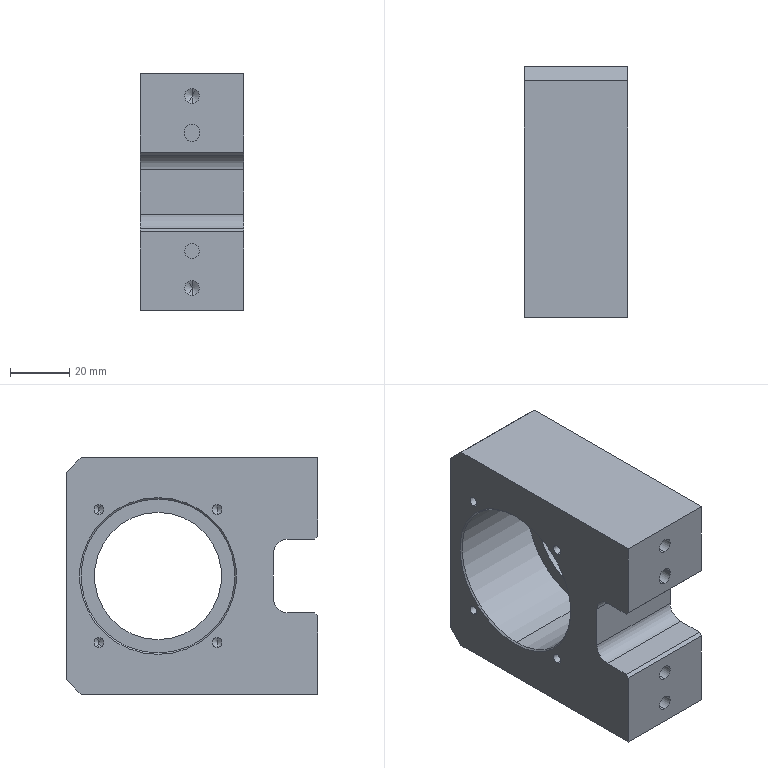Part | SolidWorks | features Chamfer 3, HoleWzd 2, Cut 1, Extrusion 1, Fillet 1, ICE 1 | 1 solid | 56 faces | box 35 x 85 x 80 mm | volume 150248 mm3 | cylinder 23 | plane 19 | cone 14 | commonest cylinder face diameters 5 x9 3.3 x8 10 x2 43 x2 52 x2
STEP:
#1=CARTESIAN_POINT('',(-17.,54.,-26.));
#2=VERTEX_POINT('',#1);
#3=CARTESIAN_POINT('',(-17.,54.,26.));
#4=VERTEX_POINT('',#3);
#5=CARTESIAN_POINT('',(-17.,54.,0.));
#6=DIRECTION('',(-1.,0.,0.));
#7=DIRECTION('',(0.,0.,1.));
#8=AXIS2_PLACEMENT_3D('',#5,#6,#7);
#9=CIRCLE('',#8,26.);
#10=EDGE_CURVE('',#2,#4,#9,.T.);
#11=ORIENTED_EDGE('',*,*,#10,.F.);
#12=CARTESIAN_POINT('',(-17.5,54.,-26.5));
#13=VERTEX_POINT('',#12);
#14=CARTESIAN_POINT('',(-17.,54.,-26.));
#15=DIRECTION('',(-0.7071,0.,-0.7071));
#16=VECTOR('',#15,1000.);
#17=LINE('',#14,#16);
#18=EDGE_CURVE('',#2,#13,#17,.T.);
#19=ORIENTED_EDGE('',*,*,#18,.T.);
#20=CARTESIAN_POINT('',(-17.5,54.,26.5));
#21=VERTEX_POINT('',#20);
#22=CARTESIAN_POINT('',(-17.5,54.,0.));
#23=DIRECTION('',(1.,0.,0.));
#24=DIRECTION('',(0.,0.,1.));
#25=AXIS2_PLACEMENT_3D('',#22,#23,#24);
#26=CIRCLE('',#25,26.5);
#27=EDGE_CURVE('',#21,#13,#26,.T.);
#28=ORIENTED_EDGE('',*,*,#27,.F.);
#29=CARTESIAN_POINT('',(-17.,54.,26.));
#30=DIRECTION('',(-0.7071,0.,0.7071));
#31=VECTOR('',#30,1000.);
#32=LINE('',#29,#31);
#33=EDGE_CURVE('',#4,#21,#32,.T.);
#34=ORIENTED_EDGE('',*,*,#33,.F.);
#35=EDGE_LOOP('',(#11,#19,#28,#34));
#36=FACE_OUTER_BOUND('',#35,.T.);
#37=CARTESIAN_POINT('',(-17.,54.,0.));
#38=DIRECTION('',(-1.,0.,0.));
#39=DIRECTION('',(0.,0.,1.));
#40=AXIS2_PLACEMENT_3D('',#37,#38,#39);
#41=CONICAL_SURFACE('',#40,26.,0.7854);
#42=ADVANCED_FACE('',(#36),#41,.F.);
#43=CARTESIAN_POINT('',(-6.,74.,-24.15));
#44=VERTEX_POINT('',#43);
#45=CARTESIAN_POINT('',(-6.,74.,-20.85));
#46=VERTEX_POINT('',#45);
#47=CARTESIAN_POINT('',(-6.,74.,-22.5));
#48=DIRECTION('',(-1.,0.,0.));
#49=DIRECTION('',(0.,0.,1.));
#50=AXIS2_PLACEMENT_3D('',#47,#48,#49);
#51=CIRCLE('',#50,1.65);
#52=EDGE_CURVE('',#44,#46,#51,.T.);
#53=ORIENTED_EDGE('',*,*,#52,.F.);
#54=CARTESIAN_POINT('',(-17.5,74.,-24.15));
#55=VERTEX_POINT('',#54);
#56=CARTESIAN_POINT('',(-17.5,74.,-24.15));
#57=DIRECTION('',(-1.,0.,0.));
#58=VECTOR('',#57,1000.);
#59=LINE('',#56,#58);
#60=EDGE_CURVE('',#44,#55,#59,.T.);
#61=ORIENTED_EDGE('',*,*,#60,.T.);
#62=CARTESIAN_POINT('',(-17.5,74.,-20.85));
#63=VERTEX_POINT('',#62);
#64=CARTESIAN_POINT('',(-17.5,74.,-22.5));
#65=DIRECTION('',(-1.,0.,0.));
#66=DIRECTION('',(0.,0.,1.));
#67=AXIS2_PLACEMENT_3D('',#64,#65,#66);
#68=CIRCLE('',#67,1.65);
#69=EDGE_CURVE('',#55,#63,#68,.T.);
#70=ORIENTED_EDGE('',*,*,#69,.T.);
#71=CARTESIAN_POINT('',(-17.5,74.,-20.85));
#72=DIRECTION('',(-1.,0.,0.));
#73=VECTOR('',#72,1000.);
#74=LINE('',#71,#73);
#75=EDGE_CURVE('',#46,#63,#74,.T.);
#76=ORIENTED_EDGE('',*,*,#75,.F.);
#77=EDGE_LOOP('',(#53,#61,#70,#76));
#78=FACE_OUTER_BOUND('',#77,.T.);
#79=CARTESIAN_POINT('',(-17.5,74.,-22.5));
#80=DIRECTION('',(-1.,0.,0.));
#81=DIRECTION('',(0.,0.,1.));
#82=AXIS2_PLACEMENT_3D('',#79,#80,#81);
#83=CYLINDRICAL_SURFACE('',#82,1.65);
#84=ADVANCED_FACE('',(#78),#83,.F.);
#85=CARTESIAN_POINT('',(-5.009,74.,-22.5));
#86=VERTEX_POINT('',#85);
#87=CARTESIAN_POINT('',(-6.,74.,-20.85));
#88=DIRECTION('',(-0.515,0.,0.8572));
#89=VECTOR('',#88,1000.);
#90=LINE('',#87,#89);
#91=EDGE_CURVE('',#86,#46,#90,.T.);
#92=ORIENTED_EDGE('',*,*,#91,.F.);
#93=CARTESIAN_POINT('',(-6.,74.,-24.15));
#94=DIRECTION('',(-0.515,0.,-0.8572));
#95=VECTOR('',#94,1000.);
#96=LINE('',#93,#95);
#97=EDGE_CURVE('',#86,#44,#96,.T.);
#98=ORIENTED_EDGE('',*,*,#97,.T.);
#99=ORIENTED_EDGE('',*,*,#52,.T.);
#100=EDGE_LOOP('',(#92,#98,#99));
#101=FACE_OUTER_BOUND('',#100,.T.);
#102=CARTESIAN_POINT('',(-6.,74.,-22.5));
#103=DIRECTION('',(-1.,0.,0.));
#104=DIRECTION('',(0.,0.,1.));
#105=AXIS2_PLACEMENT_3D('',#102,#103,#104);
#106=CONICAL_SURFACE('',#105,1.65,1.03);
#107=ADVANCED_FACE('',(#101),#106,.F.);
#108=CARTESIAN_POINT('',(-6.,74.,20.85));
#109=VERTEX_POINT('',#108);
#110=CARTESIAN_POINT('',(-6.,74.,24.15));
#111=VERTEX_POINT('',#110);
#112=CARTESIAN_POINT('',(-6.,74.,22.5));
#113=DIRECTION('',(-1.,0.,0.));
#114=DIRECTION('',(0.,0.,1.));
#115=AXIS2_PLACEMENT_3D('',#112,#113,#114);
#116=CIRCLE('',#115,1.65);
#117=EDGE_CURVE('',#109,#111,#116,.T.);
#118=ORIENTED_EDGE('',*,*,#117,.F.);
#119=CARTESIAN_POINT('',(-17.5,74.,20.85));
#120=VERTEX_POINT('',#119);
#121=CARTESIAN_POINT('',(-17.5,74.,20.85));
#122=DIRECTION('',(-1.,0.,0.));
#123=VECTOR('',#122,1000.);
#124=LINE('',#121,#123);
#125=EDGE_CURVE('',#109,#120,#124,.T.);
#126=ORIENTED_EDGE('',*,*,#125,.T.);
#127=CARTESIAN_POINT('',(-17.5,74.,24.15));
#128=VERTEX_POINT('',#127);
#129=CARTESIAN_POINT('',(-17.5,74.,22.5));
#130=DIRECTION('',(-1.,0.,0.));
#131=DIRECTION('',(0.,0.,1.));
#132=AXIS2_PLACEMENT_3D('',#129,#130,#131);
#133=CIRCLE('',#132,1.65);
#134=EDGE_CURVE('',#120,#128,#133,.T.);
#135=ORIENTED_EDGE('',*,*,#134,.T.);
#136=CARTESIAN_POINT('',(-17.5,74.,24.15));
#137=DIRECTION('',(-1.,0.,0.));
#138=VECTOR('',#137,1000.);
#139=LINE('',#136,#138);
#140=EDGE_CURVE('',#111,#128,#139,.T.);
#141=ORIENTED_EDGE('',*,*,#140,.F.);
#142=EDGE_LOOP('',(#118,#126,#135,#141));
#143=FACE_OUTER_BOUND('',#142,.T.);
#144=CARTESIAN_POINT('',(-17.5,74.,22.5));
#145=DIRECTION('',(-1.,0.,0.));
#146=DIRECTION('',(0.,0.,1.));
#147=AXIS2_PLACEMENT_3D('',#144,#145,#146);
#148=CYLINDRICAL_SURFACE('',#147,1.65);
#149=ADVANCED_FACE('',(#143),#148,.F.);
#150=CARTESIAN_POINT('',(-5.009,74.,22.5));
#151=VERTEX_POINT('',#150);
#152=CARTESIAN_POINT('',(-6.,74.,24.15));
#153=DIRECTION('',(-0.515,0.,0.8572));
#154=VECTOR('',#153,1000.);
#155=LINE('',#152,#154);
#156=EDGE_CURVE('',#151,#111,#155,.T.);
#157=ORIENTED_EDGE('',*,*,#156,.F.);
#158=CARTESIAN_POINT('',(-6.,74.,20.85));
#159=DIRECTION('',(-0.515,0.,-0.8572));
#160=VECTOR('',#159,1000.);
#161=LINE('',#158,#160);
#162=EDGE_CURVE('',#151,#109,#161,.T.);
#163=ORIENTED_EDGE('',*,*,#162,.T.);
#164=ORIENTED_EDGE('',*,*,#117,.T.);
#165=EDGE_LOOP('',(#157,#163,#164));
#166=FACE_OUTER_BOUND('',#165,.T.);
#167=CARTESIAN_POINT('',(-6.,74.,22.5));
#168=DIRECTION('',(-1.,0.,0.));
#169=DIRECTION('',(0.,0.,1.));
#170=AXIS2_PLACEMENT_3D('',#167,#168,#169);
#171=CONICAL_SURFACE('',#170,1.65,1.03);
#172=ADVANCED_FACE('',(#166),#171,.F.);
#173=CARTESIAN_POINT('',(-6.,34.,20.85));
#174=VERTEX_POINT('',#173);
#175=CARTESIAN_POINT('',(-6.,34.,24.15));
#176=VERTEX_POINT('',#175);
#177=CARTESIAN_POINT('',(-6.,34.,22.5));
#178=DIRECTION('',(-1.,0.,0.));
#179=DIRECTION('',(0.,0.,1.));
#180=AXIS2_PLACEMENT_3D('',#177,#178,#179);
#181=CIRCLE('',#180,1.65);
#182=EDGE_CURVE('',#174,#176,#181,.T.);
#183=ORIENTED_EDGE('',*,*,#182,.F.);
#184=CARTESIAN_POINT('',(-17.5,34.,20.85));
#185=VERTEX_POINT('',#184);
#186=CARTESIAN_POINT('',(-17.5,34.,20.85));
#187=DIRECTION('',(-1.,0.,0.));
#188=VECTOR('',#187,1000.);
#189=LINE('',#186,#188);
#190=EDGE_CURVE('',#174,#185,#189,.T.);
#191=ORIENTED_EDGE('',*,*,#190,.T.);
#192=CARTESIAN_POINT('',(-17.5,34.,24.15));
#193=VERTEX_POINT('',#192);
#194=CARTESIAN_POINT('',(-17.5,34.,22.5));
#195=DIRECTION('',(-1.,0.,0.));
#196=DIRECTION('',(0.,0.,1.));
#197=AXIS2_PLACEMENT_3D('',#194,#195,#196);
#198=CIRCLE('',#197,1.65);
#199=EDGE_CURVE('',#185,#193,#198,.T.);
#200=ORIENTED_EDGE('',*,*,#199,.T.);
#201=CARTESIAN_POINT('',(-17.5,34.,24.15));
#202=DIRECTION('',(-1.,0.,0.));
#203=VECTOR('',#202,1000.);
#204=LINE('',#201,#203);
#205=EDGE_CURVE('',#176,#193,#204,.T.);
#206=ORIENTED_EDGE('',*,*,#205,.F.);
#207=EDGE_LOOP('',(#183,#191,#200,#206));
#208=FACE_OUTER_BOUND('',#207,.T.);
#209=CARTESIAN_POINT('',(-17.5,34.,22.5));
#210=DIRECTION('',(-1.,0.,0.));
#211=DIRECTION('',(0.,0.,1.));
#212=AXIS2_PLACEMENT_3D('',#209,#210,#211);
#213=CYLINDRICAL_SURFACE('',#212,1.65);
#214=ADVANCED_FACE('',(#208),#213,.F.);
#215=CARTESIAN_POINT('',(-5.009,34.,22.5));
#216=VERTEX_POINT('',#215);
#217=CARTESIAN_POINT('',(-6.,34.,24.15));
#218=DIRECTION('',(-0.515,0.,0.8572));
#219=VECTOR('',#218,1000.);
#220=LINE('',#217,#219);
#221=EDGE_CURVE('',#216,#176,#220,.T.);
#222=ORIENTED_EDGE('',*,*,#221,.F.);
#223=CARTESIAN_POINT('',(-6.,34.,20.85));
#224=DIRECTION('',(-0.515,0.,-0.8572));
#225=VECTOR('',#224,1000.);
#226=LINE('',#223,#225);
#227=EDGE_CURVE('',#216,#174,#226,.T.);
#228=ORIENTED_EDGE('',*,*,#227,.T.);
#229=ORIENTED_EDGE('',*,*,#182,.T.);
#230=EDGE_LOOP('',(#222,#228,#229));
#231=FACE_OUTER_BOUND('',#230,.T.);
#232=CARTESIAN_POINT('',(-6.,34.,22.5));
#233=DIRECTION('',(-1.,0.,0.));
#234=DIRECTION('',(0.,0.,1.));
#235=AXIS2_PLACEMENT_3D('',#232,#233,#234);
#236=CONICAL_SURFACE('',#235,1.65,1.03);
#237=ADVANCED_FACE('',(#231),#236,.F.);
#238=CARTESIAN_POINT('',(-6.,34.,-24.15));
#239=VERTEX_POINT('',#238);
#240=CARTESIAN_POINT('',(-6.,34.,-20.85));
#241=VERTEX_POINT('',#240);
#242=CARTESIAN_POINT('',(-6.,34.,-22.5));
#243=DIRECTION('',(-1.,0.,0.));
#244=DIRECTION('',(0.,0.,1.));
#245=AXIS2_PLACEMENT_3D('',#242,#243,#244);
#246=CIRCLE('',#245,1.65);
#247=EDGE_CURVE('',#239,#241,#246,.T.);
#248=ORIENTED_EDGE('',*,*,#247,.F.);
#249=CARTESIAN_POINT('',(-17.5,34.,-24.15));
#250=VERTEX_POINT('',#249);
#251=CARTESIAN_POINT('',(-17.5,34.,-24.15));
#252=DIRECTION('',(-1.,0.,0.));
#253=VECTOR('',#252,1000.);
#254=LINE('',#251,#253);
#255=EDGE_CURVE('',#239,#250,#254,.T.);
#256=ORIENTED_EDGE('',*,*,#255,.T.);
#257=CARTESIAN_POINT('',(-17.5,34.,-20.85));
#258=VERTEX_POINT('',#257);
#259=CARTESIAN_POINT('',(-17.5,34.,-22.5));
#260=DIRECTION('',(-1.,0.,0.));
#261=DIRECTION('',(0.,0.,1.));
#262=AXIS2_PLACEMENT_3D('',#259,#260,#261);
#263=CIRCLE('',#262,1.65);
#264=EDGE_CURVE('',#250,#258,#263,.T.);
#265=ORIENTED_EDGE('',*,*,#264,.T.);
#266=CARTESIAN_POINT('',(-17.5,34.,-20.85));
#267=DIRECTION('',(-1.,0.,0.));
#268=VECTOR('',#267,1000.);
#269=LINE('',#266,#268);
#270=EDGE_CURVE('',#241,#258,#269,.T.);
#271=ORIENTED_EDGE('',*,*,#270,.F.);
#272=EDGE_LOOP('',(#248,#256,#265,#271));
#273=FACE_OUTER_BOUND('',#272,.T.);
#274=CARTESIAN_POINT('',(-17.5,34.,-22.5));
#275=DIRECTION('',(-1.,0.,0.));
#276=DIRECTION('',(0.,0.,1.));
#277=AXIS2_PLACEMENT_3D('',#274,#275,#276);
#278=CYLINDRICAL_SURFACE('',#277,1.65);
#279=ADVANCED_FACE('',(#273),#278,.F.);
#280=CARTESIAN_POINT('',(-5.009,34.,-22.5));
#281=VERTEX_POINT('',#280);
#282=CARTESIAN_POINT('',(-6.,34.,-20.85));
#283=DIRECTION('',(-0.515,0.,0.8572));
#284=VECTOR('',#283,1000.);
#285=LINE('',#282,#284);
#286=EDGE_CURVE('',#281,#241,#285,.T.);
#287=ORIENTED_EDGE('',*,*,#286,.F.);
#288=CARTESIAN_POINT('',(-6.,34.,-24.15));
#289=DIRECTION('',(-0.515,0.,-0.8572));
#290=VECTOR('',#289,1000.);
#291=LINE('',#288,#290);
#292=EDGE_CURVE('',#281,#239,#291,.T.);
#293=ORIENTED_EDGE('',*,*,#292,.T.);
#294=ORIENTED_EDGE('',*,*,#247,.T.);
#295=EDGE_LOOP('',(#287,#293,#294));
#296=FACE_OUTER_BOUND('',#295,.T.);
#297=CARTESIAN_POINT('',(-6.,34.,-22.5));
#298=DIRECTION('',(-1.,0.,0.));
#299=DIRECTION('',(0.,0.,1.));
#300=AXIS2_PLACEMENT_3D('',#297,#298,#299);
#301=CONICAL_SURFACE('',#300,1.65,1.03);
#302=ADVANCED_FACE('',(#296),#301,.F.);
#303=CARTESIAN_POINT('',(14.5,54.,-26.));
#304=VERTEX_POINT('',#303);
#305=CARTESIAN_POINT('',(14.5,54.,26.));
#306=VERTEX_POINT('',#305);
#307=CARTESIAN_POINT('',(14.5,54.,0.));
#308=DIRECTION('',(-1.,0.,0.));
#309=DIRECTION('',(0.,0.,1.));
#310=AXIS2_PLACEMENT_3D('',#307,#308,#309);
#311=CIRCLE('',#310,26.);
#312=EDGE_CURVE('',#304,#306,#311,.T.);
#313=ORIENTED_EDGE('',*,*,#312,.F.);
#314=CARTESIAN_POINT('',(14.5,54.,-26.));
#315=DIRECTION('',(-1.,0.,0.));
#316=VECTOR('',#315,1000.);
#317=LINE('',#314,#316);
#318=EDGE_CURVE('',#304,#2,#317,.T.);
#319=ORIENTED_EDGE('',*,*,#318,.T.);
#320=ORIENTED_EDGE('',*,*,#10,.T.);
#321=CARTESIAN_POINT('',(14.5,54.,26.));
#322=DIRECTION('',(-1.,0.,0.));
#323=VECTOR('',#322,1000.);
#324=LINE('',#321,#323);
#325=EDGE_CURVE('',#306,#4,#324,.T.);
#326=ORIENTED_EDGE('',*,*,#325,.F.);
#327=EDGE_LOOP('',(#313,#319,#320,#326));
#328=FACE_OUTER_BOUND('',#327,.T.);
#329=CARTESIAN_POINT('',(14.5,54.,0.));
#330=DIRECTION('',(-1.,0.,0.));
#331=DIRECTION('',(0.,0.,1.));
#332=AXIS2_PLACEMENT_3D('',#329,#330,#331);
#333=CYLINDRICAL_SURFACE('',#332,26.);
#334=ADVANCED_FACE('',(#328),#333,.F.);
#335=CARTESIAN_POINT('',(0.,15.,17.));
#336=VERTEX_POINT('',#335);
#337=CARTESIAN_POINT('',(2.5,15.,19.5));
#338=VERTEX_POINT('',#337);
#339=CARTESIAN_POINT('',(0.,15.,19.5));
#340=DIRECTION('',(0.,-1.,0.));
#341=DIRECTION('',(0.,0.,-1.));
#342=AXIS2_PLACEMENT_3D('',#339,#340,#341);
#343=CIRCLE('',#342,2.5);
#344=EDGE_CURVE('',#336,#338,#343,.T.);
#345=ORIENTED_EDGE('',*,*,#344,.F.);
#346=CARTESIAN_POINT('',(0.,0.,17.));
#347=VERTEX_POINT('',#346);
#348=CARTESIAN_POINT('',(0.,15.,17.));
#349=DIRECTION('',(0.,-1.,0.));
#350=VECTOR('',#349,1000.);
#351=LINE('',#348,#350);
#352=EDGE_CURVE('',#336,#347,#351,.T.);
#353=ORIENTED_EDGE('',*,*,#352,.T.);
#354=CARTESIAN_POINT('',(2.5,0.,19.5));
#355=VERTEX_POINT('',#354);
#356=CARTESIAN_POINT('',(0.,0.,19.5));
#357=DIRECTION('',(0.,-1.,0.));
#358=DIRECTION('',(0.,0.,-1.));
#359=AXIS2_PLACEMENT_3D('',#356,#357,#358);
#360=CIRCLE('',#359,2.5);
#361=EDGE_CURVE('',#347,#355,#360,.T.);
#362=ORIENTED_EDGE('',*,*,#361,.T.);
#363=CARTESIAN_POINT('',(2.5,15.,19.5));
#364=DIRECTION('',(0.,-1.,0.));
#365=VECTOR('',#364,1000.);
#366=LINE('',#363,#365);
#367=EDGE_CURVE('',#338,#355,#366,.T.);
#368=ORIENTED_EDGE('',*,*,#367,.F.);
#369=EDGE_LOOP('',(#345,#353,#362,#368));
#370=FACE_OUTER_BOUND('',#369,.T.);
#371=CARTESIAN_POINT('',(0.,15.,19.5));
#372=DIRECTION('',(0.,-1.,0.));
#373=DIRECTION('',(0.,0.,-1.));
#374=AXIS2_PLACEMENT_3D('',#371,#372,#373);
#375=CYLINDRICAL_SURFACE('',#374,2.5);
#376=ADVANCED_FACE('',(#370),#375,.F.);
#377=CARTESIAN_POINT('',(0.,15.,-17.5));
#378=VERTEX_POINT('',#377);
#379=CARTESIAN_POINT('',(0.,15.,-22.5));
#380=VERTEX_POINT('',#379);
#381=CARTESIAN_POINT('',(0.,15.,-20.));
#382=DIRECTION('',(0.,-1.,0.));
#383=DIRECTION('',(0.,0.,-1.));
#384=AXIS2_PLACEMENT_3D('',#381,#382,#383);
#385=CIRCLE('',#384,2.5);
#386=EDGE_CURVE('',#378,#380,#385,.T.);
#387=ORIENTED_EDGE('',*,*,#386,.F.);
#388=CARTESIAN_POINT('',(0.,0.,-17.5));
#389=VERTEX_POINT('',#388);
#390=CARTESIAN_POINT('',(0.,15.,-17.5));
#391=DIRECTION('',(0.,-1.,0.));
#392=VECTOR('',#391,1000.);
#393=LINE('',#390,#392);
#394=EDGE_CURVE('',#378,#389,#393,.T.);
#395=ORIENTED_EDGE('',*,*,#394,.T.);
#396=CARTESIAN_POINT('',(0.,0.,-22.5));
#397=VERTEX_POINT('',#396);
#398=CARTESIAN_POINT('',(0.,0.,-20.));
#399=DIRECTION('',(0.,-1.,0.));
#400=DIRECTION('',(0.,0.,-1.));
#401=AXIS2_PLACEMENT_3D('',#398,#399,#400);
#402=CIRCLE('',#401,2.5);
#403=EDGE_CURVE('',#389,#397,#402,.T.);
#404=ORIENTED_EDGE('',*,*,#403,.T.);
#405=CARTESIAN_POINT('',(0.,15.,-22.5));
#406=DIRECTION('',(0.,-1.,0.));
#407=VECTOR('',#406,1000.);
#408=LINE('',#405,#407);
#409=EDGE_CURVE('',#380,#397,#408,.T.);
#410=ORIENTED_EDGE('',*,*,#409,.F.);
#411=EDGE_LOOP('',(#387,#395,#404,#410));
#412=FACE_OUTER_BOUND('',#411,.T.);
#413=CARTESIAN_POINT('',(0.,15.,-20.));
#414=DIRECTION('',(0.,-1.,0.));
#415=DIRECTION('',(0.,0.,-1.));
#416=AXIS2_PLACEMENT_3D('',#413,#414,#415);
#417=CYLINDRICAL_SURFACE('',#416,2.5);
#418=ADVANCED_FACE('',(#412),#417,.F.);
#419=CARTESIAN_POINT('',(0.,17.,35.));
#420=VERTEX_POINT('',#419);
#421=CARTESIAN_POINT('',(0.,17.,30.));
#422=VERTEX_POINT('',#421);
#423=CARTESIAN_POINT('',(0.,17.,32.5));
#424=DIRECTION('',(0.,-1.,0.));
#425=DIRECTION('',(0.,0.,-1.));
#426=AXIS2_PLACEMENT_3D('',#423,#424,#425);
#427=CIRCLE('',#426,2.5);
#428=EDGE_CURVE('',#420,#422,#427,.T.);
#429=ORIENTED_EDGE('',*,*,#428,.F.);
#430=CARTESIAN_POINT('',(0.,0.,35.));
#431=VERTEX_POINT('',#430);
#432=CARTESIAN_POINT('',(0.,0.,35.));
#433=DIRECTION('',(0.,-1.,0.));
#434=VECTOR('',#433,1000.);
#435=LINE('',#432,#434);
#436=EDGE_CURVE('',#420,#431,#435,.T.);
#437=ORIENTED_EDGE('',*,*,#436,.T.);
#438=CARTESIAN_POINT('',(0.,0.,30.));
#439=VERTEX_POINT('',#438);
#440=CARTESIAN_POINT('',(0.,0.,32.5));
#441=DIRECTION('',(0.,-1.,0.));
#442=DIRECTION('',(0.,0.,-1.));
#443=AXIS2_PLACEMENT_3D('',#440,#441,#442);
#444=CIRCLE('',#443,2.5);
#445=EDGE_CURVE('',#431,#439,#444,.T.);
#446=ORIENTED_EDGE('',*,*,#445,.T.);
#447=CARTESIAN_POINT('',(0.,0.,30.));
#448=DIRECTION('',(0.,-1.,0.));
#449=VECTOR('',#448,1000.);
#450=LINE('',#447,#449);
#451=EDGE_CURVE('',#422,#439,#450,.T.);
#452=ORIENTED_EDGE('',*,*,#451,.F.);
#453=EDGE_LOOP('',(#429,#437,#446,#452));
#454=FACE_OUTER_BOUND('',#453,.T.);
#455=CARTESIAN_POINT('',(0.,0.,32.5));
#456=DIRECTION('',(0.,-1.,0.));
#457=DIRECTION('',(0.,0.,-1.));
#458=AXIS2_PLACEMENT_3D('',#455,#456,#457);
#459=CYLINDRICAL_SURFACE('',#458,2.5);
#460=ADVANCED_FACE('',(#454),#459,.F.);
#461=CARTESIAN_POINT('',(0.,18.502,32.5));
#462=VERTEX_POINT('',#461);
#463=CARTESIAN_POINT('',(0.,17.,30.));
#464=DIRECTION('',(0.,-0.515,-0.8572));
#465=VECTOR('',#464,1000.);
#466=LINE('',#463,#465);
#467=EDGE_CURVE('',#462,#422,#466,.T.);
#468=ORIENTED_EDGE('',*,*,#467,.F.);
#469=CARTESIAN_POINT('',(0.,17.,35.));
#470=DIRECTION('',(0.,-0.515,0.8572));
#471=VECTOR('',#470,1000.);
#472=LINE('',#469,#471);
#473=EDGE_CURVE('',#462,#420,#472,.T.);
#474=ORIENTED_EDGE('',*,*,#473,.T.);
#475=ORIENTED_EDGE('',*,*,#428,.T.);
#476=EDGE_LOOP('',(#468,#474,#475));
#477=FACE_OUTER_BOUND('',#476,.T.);
#478=CARTESIAN_POINT('',(0.,17.,32.5));
#479=DIRECTION('',(0.,-1.,0.));
#480=DIRECTION('',(0.,0.,-1.));
#481=AXIS2_PLACEMENT_3D('',#478,#479,#480);
#482=CONICAL_SURFACE('',#481,2.5,1.03);
#483=ADVANCED_FACE('',(#477),#482,.F.);
#484=CARTESIAN_POINT('',(0.,17.,-30.));
#485=VERTEX_POINT('',#484);
#486=CARTESIAN_POINT('',(0.,17.,-35.));
#487=VERTEX_POINT('',#486);
#488=CARTESIAN_POINT('',(0.,17.,-32.5));
#489=DIRECTION('',(0.,-1.,0.));
#490=DIRECTION('',(0.,0.,-1.));
#491=AXIS2_PLACEMENT_3D('',#488,#489,#490);
#492=CIRCLE('',#491,2.5);
#493=EDGE_CURVE('',#485,#487,#492,.T.);
#494=ORIENTED_EDGE('',*,*,#493,.F.);
#495=CARTESIAN_POINT('',(0.,0.,-30.));
#496=VERTEX_POINT('',#495);
#497=CARTESIAN_POINT('',(0.,0.,-30.));
#498=DIRECTION('',(0.,-1.,0.));
#499=VECTOR('',#498,1000.);
#500=LINE('',#497,#499);
#501=EDGE_CURVE('',#485,#496,#500,.T.);
#502=ORIENTED_EDGE('',*,*,#501,.T.);
#503=CARTESIAN_POINT('',(0.,0.,-35.));
#504=VERTEX_POINT('',#503);
#505=CARTESIAN_POINT('',(0.,0.,-32.5));
#506=DIRECTION('',(0.,-1.,0.));
#507=DIRECTION('',(0.,0.,-1.));
#508=AXIS2_PLACEMENT_3D('',#505,#506,#507);
#509=CIRCLE('',#508,2.5);
#510=EDGE_CURVE('',#496,#504,#509,.T.);
#511=ORIENTED_EDGE('',*,*,#510,.T.);
#512=CARTESIAN_POINT('',(0.,0.,-35.));
#513=DIRECTION('',(0.,-1.,0.));
#514=VECTOR('',#513,1000.);
#515=LINE('',#512,#514);
#516=EDGE_CURVE('',#487,#504,#515,.T.);
#517=ORIENTED_EDGE('',*,*,#516,.F.);
#518=EDGE_LOOP('',(#494,#502,#511,#517));
#519=FACE_OUTER_BOUND('',#518,.T.);
#520=CARTESIAN_POINT('',(0.,0.,-32.5));
#521=DIRECTION('',(0.,-1.,0.));
#522=DIRECTION('',(0.,0.,-1.));
#523=AXIS2_PLACEMENT_3D('',#520,#521,#522);
#524=CYLINDRICAL_SURFACE('',#523,2.5);
#525=ADVANCED_FACE('',(#519),#524,.F.);
#526=CARTESIAN_POINT('',(0.,18.502,-32.5));
#527=VERTEX_POINT('',#526);
#528=CARTESIAN_POINT('',(0.,17.,-35.));
#529=DIRECTION('',(0.,-0.515,-0.8572));
#530=VECTOR('',#529,1000.);
#531=LINE('',#528,#530);
#532=EDGE_CURVE('',#527,#487,#531,.T.);
#533=ORIENTED_EDGE('',*,*,#532,.F.);
#534=CARTESIAN_POINT('',(0.,17.,-30.));
#535=DIRECTION('',(0.,-0.515,0.8572));
#536=VECTOR('',#535,1000.);
#537=LINE('',#534,#536);
#538=EDGE_CURVE('',#527,#485,#537,.T.);
#539=ORIENTED_EDGE('',*,*,#538,.T.);
#540=ORIENTED_EDGE('',*,*,#493,.T.);
#541=EDGE_LOOP('',(#533,#539,#540));
#542=FACE_OUTER_BOUND('',#541,.T.);
#543=CARTESIAN_POINT('',(0.,17.,-32.5));
#544=DIRECTION('',(0.,-1.,0.));
#545=DIRECTION('',(0.,0.,-1.));
#546=AXIS2_PLACEMENT_3D('',#543,#544,#545);
#547=CONICAL_SURFACE('',#546,2.5,1.03);
#548=ADVANCED_FACE('',(#542),#547,.F.);
#549=CARTESIAN_POINT('',(17.5,54.,21.5));
#550=VERTEX_POINT('',#549);
#551=CARTESIAN_POINT('',(17.5,54.,-21.5));
#552=VERTEX_POINT('',#551);
#553=CARTESIAN_POINT('',(17.5,54.,0.));
#554=DIRECTION('',(1.,0.,0.));
#555=DIRECTION('',(0.,0.,-1.));
#556=AXIS2_PLACEMENT_3D('',#553,#554,#555);
#557=CIRCLE('',#556,21.5);
#558=EDGE_CURVE('',#550,#552,#557,.T.);
#559=ORIENTED_EDGE('',*,*,#558,.T.);
#560=CARTESIAN_POINT('',(14.5,54.,-21.5));
#561=VERTEX_POINT('',#560);
#562=CARTESIAN_POINT('',(17.5,54.,-21.5));
#563=DIRECTION('',(-1.,0.,0.));
#564=VECTOR('',#563,1000.);
#565=LINE('',#562,#564);
#566=EDGE_CURVE('',#552,#561,#565,.T.);
#567=ORIENTED_EDGE('',*,*,#566,.T.);
#568=CARTESIAN_POINT('',(14.5,54.,21.5));
#569=VERTEX_POINT('',#568);
#570=CARTESIAN_POINT('',(14.5,54.,0.));
#571=DIRECTION('',(-1.,0.,0.));
#572=DIRECTION('',(0.,0.,1.));
#573=AXIS2_PLACEMENT_3D('',#570,#571,#572);
#574=CIRCLE('',#573,21.5);
#575=EDGE_CURVE('',#561,#569,#574,.T.);
#576=ORIENTED_EDGE('',*,*,#575,.T.);
#577=CARTESIAN_POINT('',(17.5,54.,21.5));
#578=DIRECTION('',(-1.,0.,0.));
#579=VECTOR('',#578,1000.);
#580=LINE('',#577,#579);
#581=EDGE_CURVE('',#550,#569,#580,.T.);
#582=ORIENTED_EDGE('',*,*,#581,.F.);
#583=EDGE_LOOP('',(#559,#567,#576,#582));
#584=FACE_OUTER_BOUND('',#583,.T.);
#585=CARTESIAN_POINT('',(17.5,54.,0.));
#586=DIRECTION('',(-1.,0.,0.));
#587=DIRECTION('',(0.,0.,1.));
#588=AXIS2_PLACEMENT_3D('',#585,#586,#587);
#589=CYLINDRICAL_SURFACE('',#588,21.5);
#590=ADVANCED_FACE('',(#584),#589,.F.);
#591=ORIENTED_EDGE('',*,*,#566,.F.);
#592=CARTESIAN_POINT('',(17.5,54.,0.));
#593=DIRECTION('',(1.,0.,0.));
#594=DIRECTION('',(0.,0.,-1.));
#595=AXIS2_PLACEMENT_3D('',#592,#593,#594);
#596=CIRCLE('',#595,21.5);
#597=EDGE_CURVE('',#552,#550,#596,.T.);
#598=ORIENTED_EDGE('',*,*,#597,.T.);
#599=ORIENTED_EDGE('',*,*,#581,.T.);
#600=CARTESIAN_POINT('',(14.5,54.,0.));
#601=DIRECTION('',(-1.,0.,0.));
#602=DIRECTION('',(0.,0.,1.));
#603=AXIS2_PLACEMENT_3D('',#600,#601,#602);
#604=CIRCLE('',#603,21.5);
#605=EDGE_CURVE('',#569,#561,#604,.T.);
#606=ORIENTED_EDGE('',*,*,#605,.T.);
#607=EDGE_LOOP('',(#591,#598,#599,#606));
#608=FACE_OUTER_BOUND('',#607,.T.);
#609=CARTESIAN_POINT('',(17.5,54.,0.));
#610=DIRECTION('',(-1.,0.,0.));
#611=DIRECTION('',(0.,0.,1.));
#612=AXIS2_PLACEMENT_3D('',#609,#610,#611);
#613=CYLINDRICAL_SURFACE('',#612,21.5);
#614=ADVANCED_FACE('',(#608),#613,.F.);
#615=CARTESIAN_POINT('',(17.5,10.,-12.5));
#616=VERTEX_POINT('',#615);
#617=CARTESIAN_POINT('',(17.5,1.,-12.5));
#618=VERTEX_POINT('',#617);
#619=CARTESIAN_POINT('',(17.5,0.,-12.5));
#620=DIRECTION('',(0.,-1.,0.));
#621=VECTOR('',#620,1000.);
#622=LINE('',#619,#621);
#623=EDGE_CURVE('',#616,#618,#622,.T.);
#624=ORIENTED_EDGE('',*,*,#623,.T.);
#625=CARTESIAN_POINT('',(17.5,0.,-13.5));
#626=VERTEX_POINT('',#625);
#627=CARTESIAN_POINT('',(17.5,0.,-13.5));
#628=DIRECTION('',(0.,-0.7071,-0.7071));
#629=VECTOR('',#628,1000.);
#630=LINE('',#627,#629);
#631=EDGE_CURVE('',#618,#626,#630,.T.);
#632=ORIENTED_EDGE('',*,*,#631,.T.);
#633=CARTESIAN_POINT('',(17.5,0.,-40.));
#634=VERTEX_POINT('',#633);
#635=CARTESIAN_POINT('',(17.5,0.,-12.5));
#636=DIRECTION('',(0.,0.,-1.));
#637=VECTOR('',#636,1000.);
#638=LINE('',#635,#637);
#639=EDGE_CURVE('',#626,#634,#638,.T.);
#640=ORIENTED_EDGE('',*,*,#639,.T.);
#641=CARTESIAN_POINT('',(17.5,80.,-40.));
#642=VERTEX_POINT('',#641);
#643=CARTESIAN_POINT('',(17.5,0.,-40.));
#644=DIRECTION('',(0.,1.,0.));
#645=VECTOR('',#644,1000.);
#646=LINE('',#643,#645);
#647=EDGE_CURVE('',#634,#642,#646,.T.);
#648=ORIENTED_EDGE('',*,*,#647,.T.);
#649=CARTESIAN_POINT('',(17.5,85.,-35.));
#650=VERTEX_POINT('',#649);
#651=CARTESIAN_POINT('',(17.5,85.,-35.));
#652=DIRECTION('',(0.,0.7071,0.7071));
#653=VECTOR('',#652,1000.);
#654=LINE('',#651,#653);
#655=EDGE_CURVE('',#642,#650,#654,.T.);
#656=ORIENTED_EDGE('',*,*,#655,.T.);
#657=CARTESIAN_POINT('',(17.5,85.,35.));
#658=VERTEX_POINT('',#657);
#659=CARTESIAN_POINT('',(17.5,85.,40.));
#660=DIRECTION('',(0.,0.,1.));
#661=VECTOR('',#660,1000.);
#662=LINE('',#659,#661);
#663=EDGE_CURVE('',#650,#658,#662,.T.);
#664=ORIENTED_EDGE('',*,*,#663,.T.);
#665=CARTESIAN_POINT('',(17.5,80.,40.));
#666=VERTEX_POINT('',#665);
#667=CARTESIAN_POINT('',(17.5,80.,40.));
#668=DIRECTION('',(0.,-0.7071,0.7071));
#669=VECTOR('',#668,1000.);
#670=LINE('',#667,#669);
#671=EDGE_CURVE('',#658,#666,#670,.T.);
#672=ORIENTED_EDGE('',*,*,#671,.T.);
#673=CARTESIAN_POINT('',(17.5,0.,40.));
#674=VERTEX_POINT('',#673);
#675=CARTESIAN_POINT('',(17.5,0.,40.));
#676=DIRECTION('',(0.,-1.,0.));
#677=VECTOR('',#676,1000.);
#678=LINE('',#675,#677);
#679=EDGE_CURVE('',#666,#674,#678,.T.);
#680=ORIENTED_EDGE('',*,*,#679,.T.);
#681=CARTESIAN_POINT('',(17.5,0.,13.5));
#682=VERTEX_POINT('',#681);
#683=CARTESIAN_POINT('',(17.5,0.,40.));
#684=DIRECTION('',(0.,0.,-1.));
#685=VECTOR('',#684,1000.);
#686=LINE('',#683,#685);
#687=EDGE_CURVE('',#674,#682,#686,.T.);
#688=ORIENTED_EDGE('',*,*,#687,.T.);
#689=CARTESIAN_POINT('',(17.5,1.,12.5));
#690=VERTEX_POINT('',#689);
#691=CARTESIAN_POINT('',(17.5,1.,12.5));
#692=DIRECTION('',(0.,0.7071,-0.7071));
#693=VECTOR('',#692,1000.);
#694=LINE('',#691,#693);
#695=EDGE_CURVE('',#682,#690,#694,.T.);
#696=ORIENTED_EDGE('',*,*,#695,.T.);
#697=CARTESIAN_POINT('',(17.5,10.,12.5));
#698=VERTEX_POINT('',#697);
#699=CARTESIAN_POINT('',(17.5,0.,12.5));
#700=DIRECTION('',(0.,1.,0.));
#701=VECTOR('',#700,1000.);
#702=LINE('',#699,#701);
#703=EDGE_CURVE('',#690,#698,#702,.T.);
#704=ORIENTED_EDGE('',*,*,#703,.T.);
#705=CARTESIAN_POINT('',(17.5,15.,7.5));
#706=VERTEX_POINT('',#705);
#707=CARTESIAN_POINT('',(17.5,10.,7.5));
#708=DIRECTION('',(-1.,0.,0.));
#709=DIRECTION('',(0.,0.,1.));
#710=AXIS2_PLACEMENT_3D('',#707,#708,#709);
#711=CIRCLE('',#710,5.);
#712=EDGE_CURVE('',#698,#706,#711,.T.);
#713=ORIENTED_EDGE('',*,*,#712,.T.);
#714=CARTESIAN_POINT('',(17.5,15.,-7.5));
#715=VERTEX_POINT('',#714);
#716=CARTESIAN_POINT('',(17.5,15.,12.5));
#717=DIRECTION('',(0.,0.,-1.));
#718=VECTOR('',#717,1000.);
#719=LINE('',#716,#718);
#720=EDGE_CURVE('',#706,#715,#719,.T.);
#721=ORIENTED_EDGE('',*,*,#720,.T.);
#722=CARTESIAN_POINT('',(17.5,10.,-7.5));
#723=DIRECTION('',(-1.,0.,0.));
#724=DIRECTION('',(0.,0.,1.));
#725=AXIS2_PLACEMENT_3D('',#722,#723,#724);
#726=CIRCLE('',#725,5.);
#727=EDGE_CURVE('',#715,#616,#726,.T.);
#728=ORIENTED_EDGE('',*,*,#727,.T.);
#729=EDGE_LOOP('',(#624,#632,#640,#648,#656,#664,#672,#680,#688,#696,#704,#713,#721,#728));
#730=FACE_OUTER_BOUND('',#729,.T.);
#731=ORIENTED_EDGE('',*,*,#558,.F.);
#732=ORIENTED_EDGE('',*,*,#597,.F.);
#733=EDGE_LOOP('',(#731,#732));
#734=FACE_BOUND('',#733,.T.);
#735=CARTESIAN_POINT('',(17.5,0.,0.));
#736=DIRECTION('',(-1.,0.,0.));
#737=DIRECTION('',(0.,0.,1.));
#738=AXIS2_PLACEMENT_3D('',#735,#736,#737);
#739=PLANE('',#738);
#740=ADVANCED_FACE('',(#730,#734),#739,.F.);
#741=ORIENTED_EDGE('',*,*,#27,.T.);
#742=CARTESIAN_POINT('',(-17.5,54.,0.));
#743=DIRECTION('',(1.,0.,0.));
#744=DIRECTION('',(0.,0.,1.));
#745=AXIS2_PLACEMENT_3D('',#742,#743,#744);
#746=CIRCLE('',#745,26.5);
#747=EDGE_CURVE('',#13,#21,#746,.T.);
#748=ORIENTED_EDGE('',*,*,#747,.T.);
#749=EDGE_LOOP('',(#741,#748));
#750=FACE_BOUND('',#749,.T.);
#751=CARTESIAN_POINT('',(-17.5,74.,-22.5));
#752=DIRECTION('',(-1.,0.,0.));
#753=DIRECTION('',(0.,0.,1.));
#754=AXIS2_PLACEMENT_3D('',#751,#752,#753);
#755=CIRCLE('',#754,1.65);
#756=EDGE_CURVE('',#63,#55,#755,.T.);
#757=ORIENTED_EDGE('',*,*,#756,.F.);
#758=ORIENTED_EDGE('',*,*,#69,.F.);
#759=EDGE_LOOP('',(#757,#758));
#760=FACE_BOUND('',#759,.T.);
#761=CARTESIAN_POINT('',(-17.5,74.,22.5));
#762=DIRECTION('',(-1.,0.,0.));
#763=DIRECTION('',(0.,0.,1.));
#764=AXIS2_PLACEMENT_3D('',#761,#762,#763);
#765=CIRCLE('',#764,1.65);
#766=EDGE_CURVE('',#128,#120,#765,.T.);
#767=ORIENTED_EDGE('',*,*,#766,.F.);
#768=ORIENTED_EDGE('',*,*,#134,.F.);
#769=EDGE_LOOP('',(#767,#768));
#770=FACE_BOUND('',#769,.T.);
#771=CARTESIAN_POINT('',(-17.5,34.,22.5));
#772=DIRECTION('',(-1.,0.,0.));
#773=DIRECTION('',(0.,0.,1.));
#774=AXIS2_PLACEMENT_3D('',#771,#772,#773);
#775=CIRCLE('',#774,1.65);
#776=EDGE_CURVE('',#193,#185,#775,.T.);
#777=ORIENTED_EDGE('',*,*,#776,.F.);
#778=ORIENTED_EDGE('',*,*,#199,.F.);
#779=EDGE_LOOP('',(#777,#778));
#780=FACE_BOUND('',#779,.T.);
#781=CARTESIAN_POINT('',(-17.5,34.,-22.5));
#782=DIRECTION('',(-1.,0.,0.));
#783=DIRECTION('',(0.,0.,1.));
#784=AXIS2_PLACEMENT_3D('',#781,#782,#783);
#785=CIRCLE('',#784,1.65);
#786=EDGE_CURVE('',#258,#250,#785,.T.);
#787=ORIENTED_EDGE('',*,*,#786,.F.);
#788=ORIENTED_EDGE('',*,*,#264,.F.);
#789=EDGE_LOOP('',(#787,#788));
#790=FACE_BOUND('',#789,.T.);
#791=CARTESIAN_POINT('',(-17.5,0.,-13.5));
#792=VERTEX_POINT('',#791);
#793=CARTESIAN_POINT('',(-17.5,0.,-40.));
#794=VERTEX_POINT('',#793);
#795=CARTESIAN_POINT('',(-17.5,0.,-12.5));
#796=DIRECTION('',(0.,0.,-1.));
#797=VECTOR('',#796,1000.);
#798=LINE('',#795,#797);
#799=EDGE_CURVE('',#792,#794,#798,.T.);
#800=ORIENTED_EDGE('',*,*,#799,.F.);
#801=CARTESIAN_POINT('',(-17.5,1.,-12.5));
#802=VERTEX_POINT('',#801);
#803=CARTESIAN_POINT('',(-17.5,6.75,-6.75));
#804=DIRECTION('',(0.,0.7071,0.7071));
#805=VECTOR('',#804,1000.);
#806=LINE('',#803,#805);
#807=EDGE_CURVE('',#792,#802,#806,.T.);
#808=ORIENTED_EDGE('',*,*,#807,.T.);
#809=CARTESIAN_POINT('',(-17.5,10.,-12.5));
#810=VERTEX_POINT('',#809);
#811=CARTESIAN_POINT('',(-17.5,0.,-12.5));
#812=DIRECTION('',(0.,-1.,0.));
#813=VECTOR('',#812,1000.);
#814=LINE('',#811,#813);
#815=EDGE_CURVE('',#810,#802,#814,.T.);
#816=ORIENTED_EDGE('',*,*,#815,.F.);
#817=CARTESIAN_POINT('',(-17.5,15.,-7.5));
#818=VERTEX_POINT('',#817);
#819=CARTESIAN_POINT('',(-17.5,10.,-7.5));
#820=DIRECTION('',(1.,0.,0.));
#821=DIRECTION('',(0.,0.,1.));
#822=AXIS2_PLACEMENT_3D('',#819,#820,#821);
#823=CIRCLE('',#822,5.);
#824=EDGE_CURVE('',#810,#818,#823,.T.);
#825=ORIENTED_EDGE('',*,*,#824,.T.);
#826=CARTESIAN_POINT('',(-17.5,15.,7.5));
#827=VERTEX_POINT('',#826);
#828=CARTESIAN_POINT('',(-17.5,15.,12.5));
#829=DIRECTION('',(0.,0.,-1.));
#830=VECTOR('',#829,1000.);
#831=LINE('',#828,#830);
#832=EDGE_CURVE('',#827,#818,#831,.T.);
#833=ORIENTED_EDGE('',*,*,#832,.F.);
#834=CARTESIAN_POINT('',(-17.5,10.,12.5));
#835=VERTEX_POINT('',#834);
#836=CARTESIAN_POINT('',(-17.5,10.,7.5));
#837=DIRECTION('',(1.,0.,0.));
#838=DIRECTION('',(0.,0.,1.));
#839=AXIS2_PLACEMENT_3D('',#836,#837,#838);
#840=CIRCLE('',#839,5.);
#841=EDGE_CURVE('',#827,#835,#840,.T.);
#842=ORIENTED_EDGE('',*,*,#841,.T.);
#843=CARTESIAN_POINT('',(-17.5,1.,12.5));
#844=VERTEX_POINT('',#843);
#845=CARTESIAN_POINT('',(-17.5,0.,12.5));
#846=DIRECTION('',(0.,1.,0.));
#847=VECTOR('',#846,1000.);
#848=LINE('',#845,#847);
#849=EDGE_CURVE('',#844,#835,#848,.T.);
#850=ORIENTED_EDGE('',*,*,#849,.F.);
#851=CARTESIAN_POINT('',(-17.5,0.,13.5));
#852=VERTEX_POINT('',#851);
#853=CARTESIAN_POINT('',(-17.5,6.75,6.75));
#854=DIRECTION('',(0.,-0.7071,0.7071));
#855=VECTOR('',#854,1000.);
#856=LINE('',#853,#855);
#857=EDGE_CURVE('',#844,#852,#856,.T.);
#858=ORIENTED_EDGE('',*,*,#857,.T.);
#859=CARTESIAN_POINT('',(-17.5,0.,40.));
#860=VERTEX_POINT('',#859);
#861=CARTESIAN_POINT('',(-17.5,0.,40.));
#862=DIRECTION('',(0.,0.,-1.));
#863=VECTOR('',#862,1000.);
#864=LINE('',#861,#863);
#865=EDGE_CURVE('',#860,#852,#864,.T.);
#866=ORIENTED_EDGE('',*,*,#865,.F.);
#867=CARTESIAN_POINT('',(-17.5,80.,40.));
#868=VERTEX_POINT('',#867);
#869=CARTESIAN_POINT('',(-17.5,0.,40.));
#870=DIRECTION('',(0.,-1.,0.));
#871=VECTOR('',#870,1000.);
#872=LINE('',#869,#871);
#873=EDGE_CURVE('',#868,#860,#872,.T.);
#874=ORIENTED_EDGE('',*,*,#873,.F.);
#875=CARTESIAN_POINT('',(-17.5,85.,35.));
#876=VERTEX_POINT('',#875);
#877=CARTESIAN_POINT('',(-17.5,60.,60.));
#878=DIRECTION('',(0.,0.7071,-0.7071));
#879=VECTOR('',#878,1000.);
#880=LINE('',#877,#879);
#881=EDGE_CURVE('',#868,#876,#880,.T.);
#882=ORIENTED_EDGE('',*,*,#881,.T.);
#883=CARTESIAN_POINT('',(-17.5,85.,-35.));
#884=VERTEX_POINT('',#883);
#885=CARTESIAN_POINT('',(-17.5,85.,40.));
#886=DIRECTION('',(0.,0.,1.));
#887=VECTOR('',#886,1000.);
#888=LINE('',#885,#887);
#889=EDGE_CURVE('',#884,#876,#888,.T.);
#890=ORIENTED_EDGE('',*,*,#889,.F.);
#891=CARTESIAN_POINT('',(-17.5,80.,-40.));
#892=VERTEX_POINT('',#891);
#893=CARTESIAN_POINT('',(-17.5,60.,-60.));
#894=DIRECTION('',(0.,-0.7071,-0.7071));
#895=VECTOR('',#894,1000.);
#896=LINE('',#893,#895);
#897=EDGE_CURVE('',#884,#892,#896,.T.);
#898=ORIENTED_EDGE('',*,*,#897,.T.);
#899=CARTESIAN_POINT('',(-17.5,0.,-40.));
#900=DIRECTION('',(0.,1.,0.));
#901=VECTOR('',#900,1000.);
#902=LINE('',#899,#901);
#903=EDGE_CURVE('',#794,#892,#902,.T.);
#904=ORIENTED_EDGE('',*,*,#903,.F.);
#905=EDGE_LOOP('',(#800,#808,#816,#825,#833,#842,#850,#858,#866,#874,#882,#890,#898,#904));
#906=FACE_OUTER_BOUND('',#905,.T.);
#907=CARTESIAN_POINT('',(-17.5,0.,0.));
#908=DIRECTION('',(-1.,0.,0.));
#909=DIRECTION('',(0.,0.,1.));
#910=AXIS2_PLACEMENT_3D('',#907,#908,#909);
#911=PLANE('',#910);
#912=ADVANCED_FACE('',(#750,#760,#770,#780,#790,#906),#911,.T.);
#913=ORIENTED_EDGE('',*,*,#679,.F.);
#914=CARTESIAN_POINT('',(17.5,80.,40.));
#915=DIRECTION('',(-1.,0.,0.));
#916=VECTOR('',#915,1000.);
#917=LINE('',#914,#916);
#918=EDGE_CURVE('',#666,#868,#917,.T.);
#919=ORIENTED_EDGE('',*,*,#918,.T.);
#920=ORIENTED_EDGE('',*,*,#873,.T.);
#921=CARTESIAN_POINT('',(17.5,0.,40.));
#922=DIRECTION('',(-1.,0.,0.));
#923=VECTOR('',#922,1000.);
#924=LINE('',#921,#923);
#925=EDGE_CURVE('',#674,#860,#924,.T.);
#926=ORIENTED_EDGE('',*,*,#925,.F.);
#927=EDGE_LOOP('',(#913,#919,#920,#926));
#928=FACE_OUTER_BOUND('',#927,.T.);
#929=CARTESIAN_POINT('',(17.5,0.,40.));
#930=DIRECTION('',(0.,0.,-1.));
#931=DIRECTION('',(-1.,0.,0.));
#932=AXIS2_PLACEMENT_3D('',#929,#930,#931);
#933=PLANE('',#932);
#934=ADVANCED_FACE('',(#928),#933,.F.);
#935=CARTESIAN_POINT('',(-2.5,0.,20.5));
#936=VERTEX_POINT('',#935);
#937=CARTESIAN_POINT('',(-2.5,0.,19.5));
#938=VERTEX_POINT('',#937);
#939=CARTESIAN_POINT('',(-2.5,0.,20.5));
#940=DIRECTION('',(0.,0.,-1.));
#941=VECTOR('',#940,1000.);
#942=LINE('',#939,#941);
#943=EDGE_CURVE('',#936,#938,#942,.T.);
#944=ORIENTED_EDGE('',*,*,#943,.F.);
#945=CARTESIAN_POINT('',(2.5,0.,20.5));
#946=VERTEX_POINT('',#945);
#947=CARTESIAN_POINT('',(0.,0.,20.5));
#948=DIRECTION('',(0.,-1.,0.));
#949=DIRECTION('',(0.,0.,-1.));
#950=AXIS2_PLACEMENT_3D('',#947,#948,#949);
#951=CIRCLE('',#950,2.5);
#952=EDGE_CURVE('',#946,#936,#951,.T.);
#953=ORIENTED_EDGE('',*,*,#952,.F.);
#954=CARTESIAN_POINT('',(2.5,0.,20.5));
#955=DIRECTION('',(0.,0.,1.));
#956=VECTOR('',#955,1000.);
#957=LINE('',#954,#956);
#958=EDGE_CURVE('',#355,#946,#957,.T.);
#959=ORIENTED_EDGE('',*,*,#958,.F.);
#960=ORIENTED_EDGE('',*,*,#361,.F.);
#961=CARTESIAN_POINT('',(0.,0.,19.5));
#962=DIRECTION('',(0.,-1.,0.));
#963=DIRECTION('',(0.,0.,-1.));
#964=AXIS2_PLACEMENT_3D('',#961,#962,#963);
#965=CIRCLE('',#964,2.5);
#966=EDGE_CURVE('',#938,#347,#965,.T.);
#967=ORIENTED_EDGE('',*,*,#966,.F.);
#968=EDGE_LOOP('',(#944,#953,#959,#960,#967));
#969=FACE_BOUND('',#968,.T.);
#970=CARTESIAN_POINT('',(0.,0.,32.5));
#971=DIRECTION('',(0.,-1.,0.));
#972=DIRECTION('',(0.,0.,-1.));
#973=AXIS2_PLACEMENT_3D('',#970,#971,#972);
#974=CIRCLE('',#973,2.5);
#975=EDGE_CURVE('',#439,#431,#974,.T.);
#976=ORIENTED_EDGE('',*,*,#975,.F.);
#977=ORIENTED_EDGE('',*,*,#445,.F.);
#978=EDGE_LOOP('',(#976,#977));
#979=FACE_BOUND('',#978,.T.);
#980=ORIENTED_EDGE('',*,*,#865,.T.);
#981=CARTESIAN_POINT('',(17.5,0.,13.5));
#982=DIRECTION('',(1.,0.,0.));
#983=VECTOR('',#982,1000.);
#984=LINE('',#981,#983);
#985=EDGE_CURVE('',#852,#682,#984,.T.);
#986=ORIENTED_EDGE('',*,*,#985,.T.);
#987=ORIENTED_EDGE('',*,*,#687,.F.);
#988=ORIENTED_EDGE('',*,*,#925,.T.);
#989=EDGE_LOOP('',(#980,#986,#987,#988));
#990=FACE_OUTER_BOUND('',#989,.T.);
#991=CARTESIAN_POINT('',(17.5,0.,40.));
#992=DIRECTION('',(0.,1.,0.));
#993=DIRECTION('',(0.,0.,1.));
#994=AXIS2_PLACEMENT_3D('',#991,#992,#993);
#995=PLANE('',#994);
#996=ADVANCED_FACE('',(#969,#979,#990),#995,.F.);
#997=ORIENTED_EDGE('',*,*,#703,.F.);
#998=CARTESIAN_POINT('',(17.5,1.,12.5));
#999=DIRECTION('',(-1.,0.,0.));
#1000=VECTOR('',#999,1000.);
#1001=LINE('',#998,#1000);
#1002=EDGE_CURVE('',#690,#844,#1001,.T.);
#1003=ORIENTED_EDGE('',*,*,#1002,.T.);
#1004=ORIENTED_EDGE('',*,*,#849,.T.);
#1005=CARTESIAN_POINT('',(17.5,10.,12.5));
#1006=DIRECTION('',(1.,0.,0.));
#1007=VECTOR('',#1006,1000.);
#1008=LINE('',#1005,#1007);
#1009=EDGE_CURVE('',#835,#698,#1008,.T.);
#1010=ORIENTED_EDGE('',*,*,#1009,.T.);
#1011=EDGE_LOOP('',(#997,#1003,#1004,#1010));
#1012=FACE_OUTER_BOUND('',#1011,.T.);
#1013=CARTESIAN_POINT('',(17.5,0.,12.5));
#1014=DIRECTION('',(0.,0.,1.));
#1015=DIRECTION('',(1.,0.,0.));
#1016=AXIS2_PLACEMENT_3D('',#1013,#1014,#1015);
#1017=PLANE('',#1016);
#1018=ADVANCED_FACE('',(#1012),#1017,.F.);
#1019=ORIENTED_EDGE('',*,*,#832,.T.);
#1020=CARTESIAN_POINT('',(17.5,15.,-7.5));
#1021=DIRECTION('',(1.,0.,0.));
#1022=VECTOR('',#1021,1000.);
#1023=LINE('',#1020,#1022);
#1024=EDGE_CURVE('',#818,#715,#1023,.T.);
#1025=ORIENTED_EDGE('',*,*,#1024,.T.);
#1026=ORIENTED_EDGE('',*,*,#720,.F.);
#1027=CARTESIAN_POINT('',(-17.5,15.,7.5));
#1028=DIRECTION('',(-1.,0.,0.));
#1029=VECTOR('',#1028,1000.);
#1030=LINE('',#1027,#1029);
#1031=EDGE_CURVE('',#706,#827,#1030,.T.);
#1032=ORIENTED_EDGE('',*,*,#1031,.T.);
#1033=EDGE_LOOP('',(#1019,#1025,#1026,#1032));
#1034=FACE_OUTER_BOUND('',#1033,.T.);
#1035=CARTESIAN_POINT('',(17.5,15.,12.5));
#1036=DIRECTION('',(0.,1.,0.));
#1037=DIRECTION('',(0.,0.,1.));
#1038=AXIS2_PLACEMENT_3D('',#1035,#1036,#1037);
#1039=PLANE('',#1038);
#1040=ADVANCED_FACE('',(#1034),#1039,.F.);
#1041=ORIENTED_EDGE('',*,*,#815,.T.);
#1042=CARTESIAN_POINT('',(17.5,1.,-12.5));
#1043=DIRECTION('',(1.,0.,0.));
#1044=VECTOR('',#1043,1000.);
#1045=LINE('',#1042,#1044);
#1046=EDGE_CURVE('',#802,#618,#1045,.T.);
#1047=ORIENTED_EDGE('',*,*,#1046,.T.);
#1048=ORIENTED_EDGE('',*,*,#623,.F.);
#1049=CARTESIAN_POINT('',(-17.5,10.,-12.5));
#1050=DIRECTION('',(-1.,0.,0.));
#1051=VECTOR('',#1050,1000.);
#1052=LINE('',#1049,#1051);
#1053=EDGE_CURVE('',#616,#810,#1052,.T.);
#1054=ORIENTED_EDGE('',*,*,#1053,.T.);
#1055=EDGE_LOOP('',(#1041,#1047,#1048,#1054));
#1056=FACE_OUTER_BOUND('',#1055,.T.);
#1057=CARTESIAN_POINT('',(17.5,0.,-12.5));
#1058=DIRECTION('',(0.,0.,-1.));
#1059=DIRECTION('',(-1.,0.,0.));
#1060=AXIS2_PLACEMENT_3D('',#1057,#1058,#1059);
#1061=PLANE('',#1060);
#1062=ADVANCED_FACE('',(#1056),#1061,.F.);
#1063=CARTESIAN_POINT('',(0.,0.,-20.));
#1064=DIRECTION('',(0.,-1.,0.));
#1065=DIRECTION('',(0.,0.,-1.));
#1066=AXIS2_PLACEMENT_3D('',#1063,#1064,#1065);
#1067=CIRCLE('',#1066,2.5);
#1068=EDGE_CURVE('',#397,#389,#1067,.T.);
#1069=ORIENTED_EDGE('',*,*,#1068,.F.);
#1070=ORIENTED_EDGE('',*,*,#403,.F.);
#1071=EDGE_LOOP('',(#1069,#1070));
#1072=FACE_BOUND('',#1071,.T.);
#1073=CARTESIAN_POINT('',(0.,0.,-32.5));
#1074=DIRECTION('',(0.,-1.,0.));
#1075=DIRECTION('',(0.,0.,-1.));
#1076=AXIS2_PLACEMENT_3D('',#1073,#1074,#1075);
#1077=CIRCLE('',#1076,2.5);
#1078=EDGE_CURVE('',#504,#496,#1077,.T.);
#1079=ORIENTED_EDGE('',*,*,#1078,.F.);
#1080=ORIENTED_EDGE('',*,*,#510,.F.);
#1081=EDGE_LOOP('',(#1079,#1080));
#1082=FACE_BOUND('',#1081,.T.);
#1083=ORIENTED_EDGE('',*,*,#639,.F.);
#1084=CARTESIAN_POINT('',(17.5,0.,-13.5));
#1085=DIRECTION('',(-1.,0.,0.));
#1086=VECTOR('',#1085,1000.);
#1087=LINE('',#1084,#1086);
#1088=EDGE_CURVE('',#626,#792,#1087,.T.);
#1089=ORIENTED_EDGE('',*,*,#1088,.T.);
#1090=ORIENTED_EDGE('',*,*,#799,.T.);
#1091=CARTESIAN_POINT('',(17.5,0.,-40.));
#1092=DIRECTION('',(-1.,0.,0.));
#1093=VECTOR('',#1092,1000.);
#1094=LINE('',#1091,#1093);
#1095=EDGE_CURVE('',#634,#794,#1094,.T.);
#1096=ORIENTED_EDGE('',*,*,#1095,.F.);
#1097=EDGE_LOOP('',(#1083,#1089,#1090,#1096));
#1098=FACE_OUTER_BOUND('',#1097,.T.);
#1099=CARTESIAN_POINT('',(17.5,0.,-12.5));
#1100=DIRECTION('',(0.,1.,0.));
#1101=DIRECTION('',(0.,0.,1.));
#1102=AXIS2_PLACEMENT_3D('',#1099,#1100,#1101);
#1103=PLANE('',#1102);
#1104=ADVANCED_FACE('',(#1072,#1082,#1098),#1103,.F.);
#1105=ORIENTED_EDGE('',*,*,#903,.T.);
#1106=CARTESIAN_POINT('',(17.5,80.,-40.));
#1107=DIRECTION('',(1.,0.,0.));
#1108=VECTOR('',#1107,1000.);
#1109=LINE('',#1106,#1108);
#1110=EDGE_CURVE('',#892,#642,#1109,.T.);
#1111=ORIENTED_EDGE('',*,*,#1110,.T.);
#1112=ORIENTED_EDGE('',*,*,#647,.F.);
#1113=ORIENTED_EDGE('',*,*,#1095,.T.);
#1114=EDGE_LOOP('',(#1105,#1111,#1112,#1113));
#1115=FACE_OUTER_BOUND('',#1114,.T.);
#1116=CARTESIAN_POINT('',(17.5,0.,-40.));
#1117=DIRECTION('',(0.,0.,1.));
#1118=DIRECTION('',(1.,0.,0.));
#1119=AXIS2_PLACEMENT_3D('',#1116,#1117,#1118);
#1120=PLANE('',#1119);
#1121=ADVANCED_FACE('',(#1115),#1120,.F.);
#1122=ORIENTED_EDGE('',*,*,#663,.F.);
#1123=CARTESIAN_POINT('',(17.5,85.,-35.));
#1124=DIRECTION('',(-1.,0.,0.));
#1125=VECTOR('',#1124,1000.);
#1126=LINE('',#1123,#1125);
#1127=EDGE_CURVE('',#650,#884,#1126,.T.);
#1128=ORIENTED_EDGE('',*,*,#1127,.T.);
#1129=ORIENTED_EDGE('',*,*,#889,.T.);
#1130=CARTESIAN_POINT('',(17.5,85.,35.));
#1131=DIRECTION('',(1.,0.,0.));
#1132=VECTOR('',#1131,1000.);
#1133=LINE('',#1130,#1132);
#1134=EDGE_CURVE('',#876,#658,#1133,.T.);
#1135=ORIENTED_EDGE('',*,*,#1134,.T.);
#1136=EDGE_LOOP('',(#1122,#1128,#1129,#1135));
#1137=FACE_OUTER_BOUND('',#1136,.T.);
#1138=CARTESIAN_POINT('',(17.5,85.,40.));
#1139=DIRECTION('',(0.,-1.,0.));
#1140=DIRECTION('',(0.,0.,-1.));
#1141=AXIS2_PLACEMENT_3D('',#1138,#1139,#1140);
#1142=PLANE('',#1141);
#1143=ADVANCED_FACE('',(#1137),#1142,.F.);
#1144=ORIENTED_EDGE('',*,*,#655,.F.);
#1145=ORIENTED_EDGE('',*,*,#1110,.F.);
#1146=ORIENTED_EDGE('',*,*,#897,.F.);
#1147=ORIENTED_EDGE('',*,*,#1127,.F.);
#1148=EDGE_LOOP('',(#1144,#1145,#1146,#1147));
#1149=FACE_OUTER_BOUND('',#1148,.T.);
#1150=CARTESIAN_POINT('',(17.5,85.,-35.));
#1151=DIRECTION('',(0.,-0.7071,0.7071));
#1152=DIRECTION('',(-1.,0.,0.));
#1153=AXIS2_PLACEMENT_3D('',#1150,#1151,#1152);
#1154=PLANE('',#1153);
#1155=ADVANCED_FACE('',(#1149),#1154,.F.);
#1156=ORIENTED_EDGE('',*,*,#671,.F.);
#1157=ORIENTED_EDGE('',*,*,#1134,.F.);
#1158=ORIENTED_EDGE('',*,*,#881,.F.);
#1159=ORIENTED_EDGE('',*,*,#918,.F.);
#1160=EDGE_LOOP('',(#1156,#1157,#1158,#1159));
#1161=FACE_OUTER_BOUND('',#1160,.T.);
#1162=CARTESIAN_POINT('',(17.5,80.,40.));
#1163=DIRECTION('',(0.,-0.7071,-0.7071));
#1164=DIRECTION('',(-1.,0.,0.));
#1165=AXIS2_PLACEMENT_3D('',#1162,#1163,#1164);
#1166=PLANE('',#1165);
#1167=ADVANCED_FACE('',(#1161),#1166,.F.);
#1168=ORIENTED_EDGE('',*,*,#727,.F.);
#1169=ORIENTED_EDGE('',*,*,#1024,.F.);
#1170=ORIENTED_EDGE('',*,*,#824,.F.);
#1171=ORIENTED_EDGE('',*,*,#1053,.F.);
#1172=EDGE_LOOP('',(#1168,#1169,#1170,#1171));
#1173=FACE_OUTER_BOUND('',#1172,.T.);
#1174=CARTESIAN_POINT('',(17.5,10.,-7.5));
#1175=DIRECTION('',(1.,0.,0.));
#1176=DIRECTION('',(0.,0.,-1.));
#1177=AXIS2_PLACEMENT_3D('',#1174,#1175,#1176);
#1178=CYLINDRICAL_SURFACE('',#1177,5.);
#1179=ADVANCED_FACE('',(#1173),#1178,.F.);
#1180=ORIENTED_EDGE('',*,*,#712,.F.);
#1181=ORIENTED_EDGE('',*,*,#1009,.F.);
#1182=ORIENTED_EDGE('',*,*,#841,.F.);
#1183=ORIENTED_EDGE('',*,*,#1031,.F.);
#1184=EDGE_LOOP('',(#1180,#1181,#1182,#1183));
#1185=FACE_OUTER_BOUND('',#1184,.T.);
#1186=CARTESIAN_POINT('',(17.5,10.,7.5));
#1187=DIRECTION('',(1.,0.,0.));
#1188=DIRECTION('',(0.,0.,-1.));
#1189=AXIS2_PLACEMENT_3D('',#1186,#1187,#1188);
#1190=CYLINDRICAL_SURFACE('',#1189,5.);
#1191=ADVANCED_FACE('',(#1185),#1190,.F.);
#1192=ORIENTED_EDGE('',*,*,#538,.F.);
#1193=ORIENTED_EDGE('',*,*,#532,.T.);
#1194=CARTESIAN_POINT('',(0.,17.,-32.5));
#1195=DIRECTION('',(0.,-1.,0.));
#1196=DIRECTION('',(0.,0.,-1.));
#1197=AXIS2_PLACEMENT_3D('',#1194,#1195,#1196);
#1198=CIRCLE('',#1197,2.5);
#1199=EDGE_CURVE('',#487,#485,#1198,.T.);
#1200=ORIENTED_EDGE('',*,*,#1199,.T.);
#1201=EDGE_LOOP('',(#1192,#1193,#1200));
#1202=FACE_OUTER_BOUND('',#1201,.T.);
#1203=CARTESIAN_POINT('',(0.,17.,-32.5));
#1204=DIRECTION('',(0.,-1.,0.));
#1205=DIRECTION('',(0.,0.,-1.));
#1206=AXIS2_PLACEMENT_3D('',#1203,#1204,#1205);
#1207=CONICAL_SURFACE('',#1206,2.5,1.03);
#1208=ADVANCED_FACE('',(#1202),#1207,.F.);
#1209=ORIENTED_EDGE('',*,*,#501,.F.);
#1210=ORIENTED_EDGE('',*,*,#1199,.F.);
#1211=ORIENTED_EDGE('',*,*,#516,.T.);
#1212=ORIENTED_EDGE('',*,*,#1078,.T.);
#1213=EDGE_LOOP('',(#1209,#1210,#1211,#1212));
#1214=FACE_OUTER_BOUND('',#1213,.T.);
#1215=CARTESIAN_POINT('',(0.,0.,-32.5));
#1216=DIRECTION('',(0.,-1.,0.));
#1217=DIRECTION('',(0.,0.,-1.));
#1218=AXIS2_PLACEMENT_3D('',#1215,#1216,#1217);
#1219=CYLINDRICAL_SURFACE('',#1218,2.5);
#1220=ADVANCED_FACE('',(#1214),#1219,.F.);
#1221=ORIENTED_EDGE('',*,*,#473,.F.);
#1222=ORIENTED_EDGE('',*,*,#467,.T.);
#1223=CARTESIAN_POINT('',(0.,17.,32.5));
#1224=DIRECTION('',(0.,-1.,0.));
#1225=DIRECTION('',(0.,0.,-1.));
#1226=AXIS2_PLACEMENT_3D('',#1223,#1224,#1225);
#1227=CIRCLE('',#1226,2.5);
#1228=EDGE_CURVE('',#422,#420,#1227,.T.);
#1229=ORIENTED_EDGE('',*,*,#1228,.T.);
#1230=EDGE_LOOP('',(#1221,#1222,#1229));
#1231=FACE_OUTER_BOUND('',#1230,.T.);
#1232=CARTESIAN_POINT('',(0.,17.,32.5));
#1233=DIRECTION('',(0.,-1.,0.));
#1234=DIRECTION('',(0.,0.,-1.));
#1235=AXIS2_PLACEMENT_3D('',#1232,#1233,#1234);
#1236=CONICAL_SURFACE('',#1235,2.5,1.03);
#1237=ADVANCED_FACE('',(#1231),#1236,.F.);
#1238=ORIENTED_EDGE('',*,*,#436,.F.);
#1239=ORIENTED_EDGE('',*,*,#1228,.F.);
#1240=ORIENTED_EDGE('',*,*,#451,.T.);
#1241=ORIENTED_EDGE('',*,*,#975,.T.);
#1242=EDGE_LOOP('',(#1238,#1239,#1240,#1241));
#1243=FACE_OUTER_BOUND('',#1242,.T.);
#1244=CARTESIAN_POINT('',(0.,0.,32.5));
#1245=DIRECTION('',(0.,-1.,0.));
#1246=DIRECTION('',(0.,0.,-1.));
#1247=AXIS2_PLACEMENT_3D('',#1244,#1245,#1246);
#1248=CYLINDRICAL_SURFACE('',#1247,2.5);
#1249=ADVANCED_FACE('',(#1243),#1248,.F.);
#1250=ORIENTED_EDGE('',*,*,#394,.F.);
#1251=CARTESIAN_POINT('',(0.,15.,-20.));
#1252=DIRECTION('',(0.,-1.,0.));
#1253=DIRECTION('',(0.,0.,-1.));
#1254=AXIS2_PLACEMENT_3D('',#1251,#1252,#1253);
#1255=CIRCLE('',#1254,2.5);
#1256=EDGE_CURVE('',#380,#378,#1255,.T.);
#1257=ORIENTED_EDGE('',*,*,#1256,.F.);
#1258=ORIENTED_EDGE('',*,*,#409,.T.);
#1259=ORIENTED_EDGE('',*,*,#1068,.T.);
#1260=EDGE_LOOP('',(#1250,#1257,#1258,#1259));
#1261=FACE_OUTER_BOUND('',#1260,.T.);
#1262=CARTESIAN_POINT('',(0.,15.,-20.));
#1263=DIRECTION('',(0.,-1.,0.));
#1264=DIRECTION('',(0.,0.,-1.));
#1265=AXIS2_PLACEMENT_3D('',#1262,#1263,#1264);
#1266=CYLINDRICAL_SURFACE('',#1265,2.5);
#1267=ADVANCED_FACE('',(#1261),#1266,.F.);
#1268=ORIENTED_EDGE('',*,*,#1256,.T.);
#1269=ORIENTED_EDGE('',*,*,#386,.T.);
#1270=EDGE_LOOP('',(#1268,#1269));
#1271=FACE_OUTER_BOUND('',#1270,.T.);
#1272=CARTESIAN_POINT('',(0.,15.,-20.));
#1273=DIRECTION('',(0.,-1.,0.));
#1274=DIRECTION('',(0.,0.,-1.));
#1275=AXIS2_PLACEMENT_3D('',#1272,#1273,#1274);
#1276=PLANE('',#1275);
#1277=ADVANCED_FACE('',(#1271),#1276,.T.);
#1278=ORIENTED_EDGE('',*,*,#952,.T.);
#1279=CARTESIAN_POINT('',(-2.5,15.,20.5));
#1280=VERTEX_POINT('',#1279);
#1281=CARTESIAN_POINT('',(-2.5,15.,20.5));
#1282=DIRECTION('',(0.,-1.,0.));
#1283=VECTOR('',#1282,1000.);
#1284=LINE('',#1281,#1283);
#1285=EDGE_CURVE('',#1280,#936,#1284,.T.);
#1286=ORIENTED_EDGE('',*,*,#1285,.F.);
#1287=CARTESIAN_POINT('',(2.5,15.,20.5));
#1288=VERTEX_POINT('',#1287);
#1289=CARTESIAN_POINT('',(0.,15.,20.5));
#1290=DIRECTION('',(0.,-1.,0.));
#1291=DIRECTION('',(0.,0.,-1.));
#1292=AXIS2_PLACEMENT_3D('',#1289,#1290,#1291);
#1293=CIRCLE('',#1292,2.5);
#1294=EDGE_CURVE('',#1288,#1280,#1293,.T.);
#1295=ORIENTED_EDGE('',*,*,#1294,.F.);
#1296=CARTESIAN_POINT('',(2.5,15.,20.5));
#1297=DIRECTION('',(0.,-1.,0.));
#1298=VECTOR('',#1297,1000.);
#1299=LINE('',#1296,#1298);
#1300=EDGE_CURVE('',#1288,#946,#1299,.T.);
#1301=ORIENTED_EDGE('',*,*,#1300,.T.);
#1302=EDGE_LOOP('',(#1278,#1286,#1295,#1301));
#1303=FACE_OUTER_BOUND('',#1302,.T.);
#1304=CARTESIAN_POINT('',(0.,15.,20.5));
#1305=DIRECTION('',(0.,-1.,0.));
#1306=DIRECTION('',(0.,0.,-1.));
#1307=AXIS2_PLACEMENT_3D('',#1304,#1305,#1306);
#1308=CYLINDRICAL_SURFACE('',#1307,2.5);
#1309=ADVANCED_FACE('',(#1303),#1308,.F.);
#1310=ORIENTED_EDGE('',*,*,#958,.T.);
#1311=ORIENTED_EDGE('',*,*,#1300,.F.);
#1312=CARTESIAN_POINT('',(2.5,15.,20.5));
#1313=DIRECTION('',(0.,0.,1.));
#1314=VECTOR('',#1313,1000.);
#1315=LINE('',#1312,#1314);
#1316=EDGE_CURVE('',#338,#1288,#1315,.T.);
#1317=ORIENTED_EDGE('',*,*,#1316,.F.);
#1318=ORIENTED_EDGE('',*,*,#367,.T.);
#1319=EDGE_LOOP('',(#1310,#1311,#1317,#1318));
#1320=FACE_OUTER_BOUND('',#1319,.T.);
#1321=CARTESIAN_POINT('',(2.5,15.,20.5));
#1322=DIRECTION('',(1.,0.,0.));
#1323=DIRECTION('',(0.,0.,-1.));
#1324=AXIS2_PLACEMENT_3D('',#1321,#1322,#1323);
#1325=PLANE('',#1324);
#1326=ADVANCED_FACE('',(#1320),#1325,.F.);
#1327=ORIENTED_EDGE('',*,*,#352,.F.);
#1328=CARTESIAN_POINT('',(-2.5,15.,19.5));
#1329=VERTEX_POINT('',#1328);
#1330=CARTESIAN_POINT('',(0.,15.,19.5));
#1331=DIRECTION('',(0.,-1.,0.));
#1332=DIRECTION('',(0.,0.,-1.));
#1333=AXIS2_PLACEMENT_3D('',#1330,#1331,#1332);
#1334=CIRCLE('',#1333,2.5);
#1335=EDGE_CURVE('',#1329,#336,#1334,.T.);
#1336=ORIENTED_EDGE('',*,*,#1335,.F.);
#1337=CARTESIAN_POINT('',(-2.5,15.,19.5));
#1338=DIRECTION('',(0.,-1.,0.));
#1339=VECTOR('',#1338,1000.);
#1340=LINE('',#1337,#1339);
#1341=EDGE_CURVE('',#1329,#938,#1340,.T.);
#1342=ORIENTED_EDGE('',*,*,#1341,.T.);
#1343=ORIENTED_EDGE('',*,*,#966,.T.);
#1344=EDGE_LOOP('',(#1327,#1336,#1342,#1343));
#1345=FACE_OUTER_BOUND('',#1344,.T.);
#1346=CARTESIAN_POINT('',(0.,15.,19.5));
#1347=DIRECTION('',(0.,-1.,0.));
#1348=DIRECTION('',(0.,0.,-1.));
#1349=AXIS2_PLACEMENT_3D('',#1346,#1347,#1348);
#1350=CYLINDRICAL_SURFACE('',#1349,2.5);
#1351=ADVANCED_FACE('',(#1345),#1350,.F.);
#1352=ORIENTED_EDGE('',*,*,#943,.T.);
#1353=ORIENTED_EDGE('',*,*,#1341,.F.);
#1354=CARTESIAN_POINT('',(-2.5,15.,20.5));
#1355=DIRECTION('',(0.,0.,-1.));
#1356=VECTOR('',#1355,1000.);
#1357=LINE('',#1354,#1356);
#1358=EDGE_CURVE('',#1280,#1329,#1357,.T.);
#1359=ORIENTED_EDGE('',*,*,#1358,.F.);
#1360=ORIENTED_EDGE('',*,*,#1285,.T.);
#1361=EDGE_LOOP('',(#1352,#1353,#1359,#1360));
#1362=FACE_OUTER_BOUND('',#1361,.T.);
#1363=CARTESIAN_POINT('',(-2.5,15.,20.5));
#1364=DIRECTION('',(-1.,0.,0.));
#1365=DIRECTION('',(0.,0.,1.));
#1366=AXIS2_PLACEMENT_3D('',#1363,#1364,#1365);
#1367=PLANE('',#1366);
#1368=ADVANCED_FACE('',(#1362),#1367,.F.);
#1369=ORIENTED_EDGE('',*,*,#1294,.T.);
#1370=ORIENTED_EDGE('',*,*,#1358,.T.);
#1371=ORIENTED_EDGE('',*,*,#1335,.T.);
#1372=ORIENTED_EDGE('',*,*,#344,.T.);
#1373=ORIENTED_EDGE('',*,*,#1316,.T.);
#1374=EDGE_LOOP('',(#1369,#1370,#1371,#1372,#1373));
#1375=FACE_OUTER_BOUND('',#1374,.T.);
#1376=CARTESIAN_POINT('',(0.,15.,20.5));
#1377=DIRECTION('',(0.,-1.,0.));
#1378=DIRECTION('',(0.,0.,-1.));
#1379=AXIS2_PLACEMENT_3D('',#1376,#1377,#1378);
#1380=PLANE('',#1379);
#1381=ADVANCED_FACE('',(#1375),#1380,.T.);
#1382=ORIENTED_EDGE('',*,*,#631,.F.);
#1383=ORIENTED_EDGE('',*,*,#1046,.F.);
#1384=ORIENTED_EDGE('',*,*,#807,.F.);
#1385=ORIENTED_EDGE('',*,*,#1088,.F.);
#1386=EDGE_LOOP('',(#1382,#1383,#1384,#1385));
#1387=FACE_OUTER_BOUND('',#1386,.T.);
#1388=CARTESIAN_POINT('',(17.5,0.,-13.5));
#1389=DIRECTION('',(0.,0.7071,-0.7071));
#1390=DIRECTION('',(-1.,0.,0.));
#1391=AXIS2_PLACEMENT_3D('',#1388,#1389,#1390);
#1392=PLANE('',#1391);
#1393=ADVANCED_FACE('',(#1387),#1392,.F.);
#1394=ORIENTED_EDGE('',*,*,#695,.F.);
#1395=ORIENTED_EDGE('',*,*,#985,.F.);
#1396=ORIENTED_EDGE('',*,*,#857,.F.);
#1397=ORIENTED_EDGE('',*,*,#1002,.F.);
#1398=EDGE_LOOP('',(#1394,#1395,#1396,#1397));
#1399=FACE_OUTER_BOUND('',#1398,.T.);
#1400=CARTESIAN_POINT('',(17.5,1.,12.5));
#1401=DIRECTION('',(0.,0.7071,0.7071));
#1402=DIRECTION('',(-1.,0.,0.));
#1403=AXIS2_PLACEMENT_3D('',#1400,#1401,#1402);
#1404=PLANE('',#1403);
#1405=ADVANCED_FACE('',(#1399),#1404,.F.);
#1406=ORIENTED_EDGE('',*,*,#318,.F.);
#1407=CARTESIAN_POINT('',(14.5,54.,0.));
#1408=DIRECTION('',(-1.,0.,0.));
#1409=DIRECTION('',(0.,0.,1.));
#1410=AXIS2_PLACEMENT_3D('',#1407,#1408,#1409);
#1411=CIRCLE('',#1410,26.);
#1412=EDGE_CURVE('',#306,#304,#1411,.T.);
#1413=ORIENTED_EDGE('',*,*,#1412,.F.);
#1414=ORIENTED_EDGE('',*,*,#325,.T.);
#1415=CARTESIAN_POINT('',(-17.,54.,0.));
#1416=DIRECTION('',(-1.,0.,0.));
#1417=DIRECTION('',(0.,0.,1.));
#1418=AXIS2_PLACEMENT_3D('',#1415,#1416,#1417);
#1419=CIRCLE('',#1418,26.);
#1420=EDGE_CURVE('',#4,#2,#1419,.T.);
#1421=ORIENTED_EDGE('',*,*,#1420,.T.);
#1422=EDGE_LOOP('',(#1406,#1413,#1414,#1421));
#1423=FACE_OUTER_BOUND('',#1422,.T.);
#1424=CARTESIAN_POINT('',(14.5,54.,0.));
#1425=DIRECTION('',(-1.,0.,0.));
#1426=DIRECTION('',(0.,0.,1.));
#1427=AXIS2_PLACEMENT_3D('',#1424,#1425,#1426);
#1428=CYLINDRICAL_SURFACE('',#1427,26.);
#1429=ADVANCED_FACE('',(#1423),#1428,.F.);
#1430=ORIENTED_EDGE('',*,*,#605,.F.);
#1431=ORIENTED_EDGE('',*,*,#575,.F.);
#1432=EDGE_LOOP('',(#1430,#1431));
#1433=FACE_BOUND('',#1432,.T.);
#1434=ORIENTED_EDGE('',*,*,#1412,.T.);
#1435=ORIENTED_EDGE('',*,*,#312,.T.);
#1436=EDGE_LOOP('',(#1434,#1435));
#1437=FACE_OUTER_BOUND('',#1436,.T.);
#1438=CARTESIAN_POINT('',(14.5,54.,0.));
#1439=DIRECTION('',(-1.,0.,0.));
#1440=DIRECTION('',(0.,0.,1.));
#1441=AXIS2_PLACEMENT_3D('',#1438,#1439,#1440);
#1442=PLANE('',#1441);
#1443=ADVANCED_FACE('',(#1433,#1437),#1442,.T.);
#1444=ORIENTED_EDGE('',*,*,#292,.F.);
#1445=ORIENTED_EDGE('',*,*,#286,.T.);
#1446=CARTESIAN_POINT('',(-6.,34.,-22.5));
#1447=DIRECTION('',(-1.,0.,0.));
#1448=DIRECTION('',(0.,0.,1.));
#1449=AXIS2_PLACEMENT_3D('',#1446,#1447,#1448);
#1450=CIRCLE('',#1449,1.65);
#1451=EDGE_CURVE('',#241,#239,#1450,.T.);
#1452=ORIENTED_EDGE('',*,*,#1451,.T.);
#1453=EDGE_LOOP('',(#1444,#1445,#1452));
#1454=FACE_OUTER_BOUND('',#1453,.T.);
#1455=CARTESIAN_POINT('',(-6.,34.,-22.5));
#1456=DIRECTION('',(-1.,0.,0.));
#1457=DIRECTION('',(0.,0.,1.));
#1458=AXIS2_PLACEMENT_3D('',#1455,#1456,#1457);
#1459=CONICAL_SURFACE('',#1458,1.65,1.03);
#1460=ADVANCED_FACE('',(#1454),#1459,.F.);
#1461=ORIENTED_EDGE('',*,*,#255,.F.);
#1462=ORIENTED_EDGE('',*,*,#1451,.F.);
#1463=ORIENTED_EDGE('',*,*,#270,.T.);
#1464=ORIENTED_EDGE('',*,*,#786,.T.);
#1465=EDGE_LOOP('',(#1461,#1462,#1463,#1464));
#1466=FACE_OUTER_BOUND('',#1465,.T.);
#1467=CARTESIAN_POINT('',(-17.5,34.,-22.5));
#1468=DIRECTION('',(-1.,0.,0.));
#1469=DIRECTION('',(0.,0.,1.));
#1470=AXIS2_PLACEMENT_3D('',#1467,#1468,#1469);
#1471=CYLINDRICAL_SURFACE('',#1470,1.65);
#1472=ADVANCED_FACE('',(#1466),#1471,.F.);
#1473=ORIENTED_EDGE('',*,*,#227,.F.);
#1474=ORIENTED_EDGE('',*,*,#221,.T.);
#1475=CARTESIAN_POINT('',(-6.,34.,22.5));
#1476=DIRECTION('',(-1.,0.,0.));
#1477=DIRECTION('',(0.,0.,1.));
#1478=AXIS2_PLACEMENT_3D('',#1475,#1476,#1477);
#1479=CIRCLE('',#1478,1.65);
#1480=EDGE_CURVE('',#176,#174,#1479,.T.);
#1481=ORIENTED_EDGE('',*,*,#1480,.T.);
#1482=EDGE_LOOP('',(#1473,#1474,#1481));
#1483=FACE_OUTER_BOUND('',#1482,.T.);
#1484=CARTESIAN_POINT('',(-6.,34.,22.5));
#1485=DIRECTION('',(-1.,0.,0.));
#1486=DIRECTION('',(0.,0.,1.));
#1487=AXIS2_PLACEMENT_3D('',#1484,#1485,#1486);
#1488=CONICAL_SURFACE('',#1487,1.65,1.03);
#1489=ADVANCED_FACE('',(#1483),#1488,.F.);
#1490=ORIENTED_EDGE('',*,*,#190,.F.);
#1491=ORIENTED_EDGE('',*,*,#1480,.F.);
#1492=ORIENTED_EDGE('',*,*,#205,.T.);
#1493=ORIENTED_EDGE('',*,*,#776,.T.);
#1494=EDGE_LOOP('',(#1490,#1491,#1492,#1493));
#1495=FACE_OUTER_BOUND('',#1494,.T.);
#1496=CARTESIAN_POINT('',(-17.5,34.,22.5));
#1497=DIRECTION('',(-1.,0.,0.));
#1498=DIRECTION('',(0.,0.,1.));
#1499=AXIS2_PLACEMENT_3D('',#1496,#1497,#1498);
#1500=CYLINDRICAL_SURFACE('',#1499,1.65);
#1501=ADVANCED_FACE('',(#1495),#1500,.F.);
#1502=ORIENTED_EDGE('',*,*,#162,.F.);
#1503=ORIENTED_EDGE('',*,*,#156,.T.);
#1504=CARTESIAN_POINT('',(-6.,74.,22.5));
#1505=DIRECTION('',(-1.,0.,0.));
#1506=DIRECTION('',(0.,0.,1.));
#1507=AXIS2_PLACEMENT_3D('',#1504,#1505,#1506);
#1508=CIRCLE('',#1507,1.65);
#1509=EDGE_CURVE('',#111,#109,#1508,.T.);
#1510=ORIENTED_EDGE('',*,*,#1509,.T.);
#1511=EDGE_LOOP('',(#1502,#1503,#1510));
#1512=FACE_OUTER_BOUND('',#1511,.T.);
#1513=CARTESIAN_POINT('',(-6.,74.,22.5));
#1514=DIRECTION('',(-1.,0.,0.));
#1515=DIRECTION('',(0.,0.,1.));
#1516=AXIS2_PLACEMENT_3D('',#1513,#1514,#1515);
#1517=CONICAL_SURFACE('',#1516,1.65,1.03);
#1518=ADVANCED_FACE('',(#1512),#1517,.F.);
#1519=ORIENTED_EDGE('',*,*,#125,.F.);
#1520=ORIENTED_EDGE('',*,*,#1509,.F.);
#1521=ORIENTED_EDGE('',*,*,#140,.T.);
#1522=ORIENTED_EDGE('',*,*,#766,.T.);
#1523=EDGE_LOOP('',(#1519,#1520,#1521,#1522));
#1524=FACE_OUTER_BOUND('',#1523,.T.);
#1525=CARTESIAN_POINT('',(-17.5,74.,22.5));
#1526=DIRECTION('',(-1.,0.,0.));
#1527=DIRECTION('',(0.,0.,1.));
#1528=AXIS2_PLACEMENT_3D('',#1525,#1526,#1527);
#1529=CYLINDRICAL_SURFACE('',#1528,1.65);
#1530=ADVANCED_FACE('',(#1524),#1529,.F.);
#1531=ORIENTED_EDGE('',*,*,#97,.F.);
#1532=ORIENTED_EDGE('',*,*,#91,.T.);
#1533=CARTESIAN_POINT('',(-6.,74.,-22.5));
#1534=DIRECTION('',(-1.,0.,0.));
#1535=DIRECTION('',(0.,0.,1.));
#1536=AXIS2_PLACEMENT_3D('',#1533,#1534,#1535);
#1537=CIRCLE('',#1536,1.65);
#1538=EDGE_CURVE('',#46,#44,#1537,.T.);
#1539=ORIENTED_EDGE('',*,*,#1538,.T.);
#1540=EDGE_LOOP('',(#1531,#1532,#1539));
#1541=FACE_OUTER_BOUND('',#1540,.T.);
#1542=CARTESIAN_POINT('',(-6.,74.,-22.5));
#1543=DIRECTION('',(-1.,0.,0.));
#1544=DIRECTION('',(0.,0.,1.));
#1545=AXIS2_PLACEMENT_3D('',#1542,#1543,#1544);
#1546=CONICAL_SURFACE('',#1545,1.65,1.03);
#1547=ADVANCED_FACE('',(#1541),#1546,.F.);
#1548=ORIENTED_EDGE('',*,*,#60,.F.);
#1549=ORIENTED_EDGE('',*,*,#1538,.F.);
#1550=ORIENTED_EDGE('',*,*,#75,.T.);
#1551=ORIENTED_EDGE('',*,*,#756,.T.);
#1552=EDGE_LOOP('',(#1548,#1549,#1550,#1551));
#1553=FACE_OUTER_BOUND('',#1552,.T.);
#1554=CARTESIAN_POINT('',(-17.5,74.,-22.5));
#1555=DIRECTION('',(-1.,0.,0.));
#1556=DIRECTION('',(0.,0.,1.));
#1557=AXIS2_PLACEMENT_3D('',#1554,#1555,#1556);
#1558=CYLINDRICAL_SURFACE('',#1557,1.65);
#1559=ADVANCED_FACE('',(#1553),#1558,.F.);
#1560=ORIENTED_EDGE('',*,*,#18,.F.);
#1561=ORIENTED_EDGE('',*,*,#1420,.F.);
#1562=ORIENTED_EDGE('',*,*,#33,.T.);
#1563=ORIENTED_EDGE('',*,*,#747,.F.);
#1564=EDGE_LOOP('',(#1560,#1561,#1562,#1563));
#1565=FACE_OUTER_BOUND('',#1564,.T.);
#1566=CARTESIAN_POINT('',(-17.,54.,0.));
#1567=DIRECTION('',(-1.,0.,0.));
#1568=DIRECTION('',(0.,0.,1.));
#1569=AXIS2_PLACEMENT_3D('',#1566,#1567,#1568);
#1570=CONICAL_SURFACE('',#1569,26.,0.7854);
#1571=ADVANCED_FACE('',(#1565),#1570,.F.);
#1572=CLOSED_SHELL('',(#42,#84,#107,#149,#172,#214,#237,#279,#302,#334,#376,#418,#460,#483,#525,#548,#590,#614,#740,#912,#934,#996,#1018,#1040,#1062,#1104,#1121,#1143,#1155,#1167,#1179,#1191,#1208,#1220,#1237,#1249,#1267,#1277,#1309,#1326,#1351,#1368,#1381,#1393,#1405,#1429,#1443,#1460,#1472,#1489,#1501,#1518,#1530,#1547,#1559,#1571));
#1573=MANIFOLD_SOLID_BREP('',#1572);
#1574=CARTESIAN_POINT('',(0.,0.,0.));
#1575=DIRECTION('',(0.,0.,1.));
#1576=DIRECTION('',(1.,0.,0.));
#1577=AXIS2_PLACEMENT_3D('',#1574,#1575,#1576);
#1578=(LENGTH_UNIT()NAMED_UNIT(*)SI_UNIT(.MILLI.,.METRE.));
#1579=UNCERTAINTY_MEASURE_WITH_UNIT(LENGTH_MEASURE(0.00001),#1578,'','');
#1580=(NAMED_UNIT(*)PLANE_ANGLE_UNIT()SI_UNIT($,.RADIAN.));
#1581=(NAMED_UNIT(*)SI_UNIT($,.STERADIAN.)SOLID_ANGLE_UNIT());
#1582=(GEOMETRIC_REPRESENTATION_CONTEXT(3)GLOBAL_UNCERTAINTY_ASSIGNED_CONTEXT((#1579))GLOBAL_UNIT_ASSIGNED_CONTEXT((#1578,#1580,#1581))REPRESENTATION_CONTEXT('',''));
#1583=ADVANCED_BREP_SHAPE_REPRESENTATION('',(#1573,#1577),#1582);